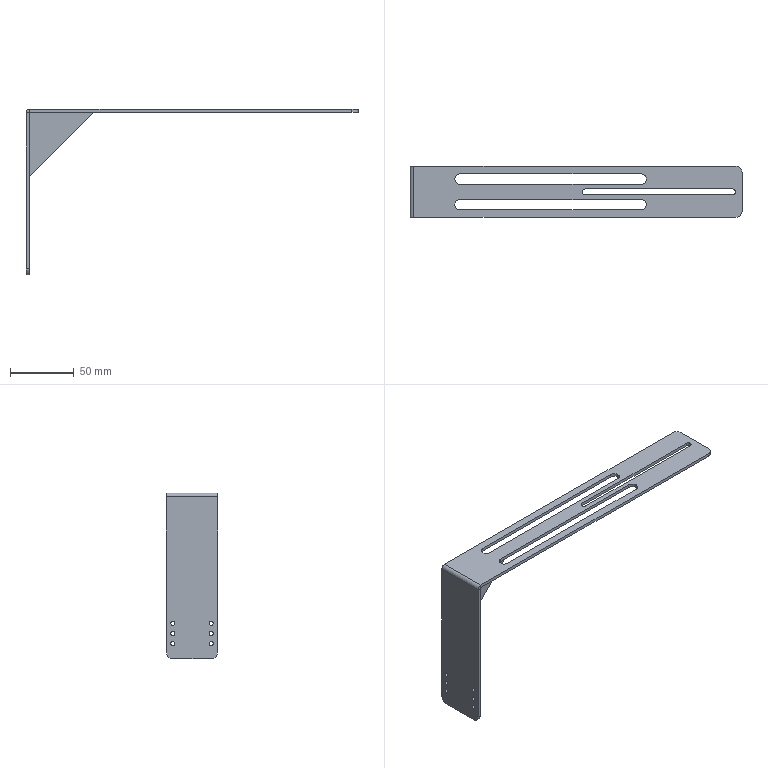Part | SolidWorks | features HoleWzd 3, EdgeFlange 1, Fillet 1, FlatPattern 1, ICE 1, SMBaseFlange 1, SheetMetal 1 | 1 solid | 49 faces | box 260 x 40 x 130 mm | volume 34410 mm3 | cylinder 28 | plane 21 | commonest cylinder face diameters 3.3 x12 8 x6 10 x4 4.5 x3 1 x2 6 x1
STEP:
#1=CARTESIAN_POINT('',(-127.5,-15.,-111.65));
#2=VERTEX_POINT('',#1);
#3=CARTESIAN_POINT('',(-127.5,-15.,-108.35));
#4=VERTEX_POINT('',#3);
#5=CARTESIAN_POINT('',(-127.5,-15.,-110.));
#6=DIRECTION('',(-1.,0.,0.));
#7=DIRECTION('',(0.,0.,1.));
#8=AXIS2_PLACEMENT_3D('',#5,#6,#7);
#9=CIRCLE('',#8,1.65);
#10=EDGE_CURVE('',#2,#4,#9,.T.);
#11=ORIENTED_EDGE('',*,*,#10,.F.);
#12=CARTESIAN_POINT('',(-130.,-15.,-111.65));
#13=VERTEX_POINT('',#12);
#14=CARTESIAN_POINT('',(-130.,-15.,-111.65));
#15=DIRECTION('',(-1.,0.,0.));
#16=VECTOR('',#15,1000.);
#17=LINE('',#14,#16);
#18=EDGE_CURVE('',#2,#13,#17,.T.);
#19=ORIENTED_EDGE('',*,*,#18,.T.);
#20=CARTESIAN_POINT('',(-130.,-15.,-108.35));
#21=VERTEX_POINT('',#20);
#22=CARTESIAN_POINT('',(-130.,-15.,-110.));
#23=DIRECTION('',(-1.,0.,0.));
#24=DIRECTION('',(0.,0.,1.));
#25=AXIS2_PLACEMENT_3D('',#22,#23,#24);
#26=CIRCLE('',#25,1.65);
#27=EDGE_CURVE('',#13,#21,#26,.T.);
#28=ORIENTED_EDGE('',*,*,#27,.T.);
#29=CARTESIAN_POINT('',(-130.,-15.,-108.35));
#30=DIRECTION('',(-1.,0.,0.));
#31=VECTOR('',#30,1000.);
#32=LINE('',#29,#31);
#33=EDGE_CURVE('',#4,#21,#32,.T.);
#34=ORIENTED_EDGE('',*,*,#33,.F.);
#35=EDGE_LOOP('',(#11,#19,#28,#34));
#36=FACE_OUTER_BOUND('',#35,.T.);
#37=CARTESIAN_POINT('',(-130.,-15.,-110.));
#38=DIRECTION('',(-1.,0.,0.));
#39=DIRECTION('',(0.,0.,1.));
#40=AXIS2_PLACEMENT_3D('',#37,#38,#39);
#41=CYLINDRICAL_SURFACE('',#40,1.65);
#42=ADVANCED_FACE('',(#36),#41,.F.);
#43=CARTESIAN_POINT('',(-127.5,15.,-111.65));
#44=VERTEX_POINT('',#43);
#45=CARTESIAN_POINT('',(-127.5,15.,-108.35));
#46=VERTEX_POINT('',#45);
#47=CARTESIAN_POINT('',(-127.5,15.,-110.));
#48=DIRECTION('',(-1.,0.,0.));
#49=DIRECTION('',(0.,0.,1.));
#50=AXIS2_PLACEMENT_3D('',#47,#48,#49);
#51=CIRCLE('',#50,1.65);
#52=EDGE_CURVE('',#44,#46,#51,.T.);
#53=ORIENTED_EDGE('',*,*,#52,.F.);
#54=CARTESIAN_POINT('',(-130.,15.,-111.65));
#55=VERTEX_POINT('',#54);
#56=CARTESIAN_POINT('',(-130.,15.,-111.65));
#57=DIRECTION('',(-1.,0.,0.));
#58=VECTOR('',#57,1000.);
#59=LINE('',#56,#58);
#60=EDGE_CURVE('',#44,#55,#59,.T.);
#61=ORIENTED_EDGE('',*,*,#60,.T.);
#62=CARTESIAN_POINT('',(-130.,15.,-108.35));
#63=VERTEX_POINT('',#62);
#64=CARTESIAN_POINT('',(-130.,15.,-110.));
#65=DIRECTION('',(-1.,0.,0.));
#66=DIRECTION('',(0.,0.,1.));
#67=AXIS2_PLACEMENT_3D('',#64,#65,#66);
#68=CIRCLE('',#67,1.65);
#69=EDGE_CURVE('',#55,#63,#68,.T.);
#70=ORIENTED_EDGE('',*,*,#69,.T.);
#71=CARTESIAN_POINT('',(-130.,15.,-108.35));
#72=DIRECTION('',(-1.,0.,0.));
#73=VECTOR('',#72,1000.);
#74=LINE('',#71,#73);
#75=EDGE_CURVE('',#46,#63,#74,.T.);
#76=ORIENTED_EDGE('',*,*,#75,.F.);
#77=EDGE_LOOP('',(#53,#61,#70,#76));
#78=FACE_OUTER_BOUND('',#77,.T.);
#79=CARTESIAN_POINT('',(-130.,15.,-110.));
#80=DIRECTION('',(-1.,0.,0.));
#81=DIRECTION('',(0.,0.,1.));
#82=AXIS2_PLACEMENT_3D('',#79,#80,#81);
#83=CYLINDRICAL_SURFACE('',#82,1.65);
#84=ADVANCED_FACE('',(#78),#83,.F.);
#85=CARTESIAN_POINT('',(-127.5,-15.,-103.65));
#86=VERTEX_POINT('',#85);
#87=CARTESIAN_POINT('',(-127.5,-15.,-100.35));
#88=VERTEX_POINT('',#87);
#89=CARTESIAN_POINT('',(-127.5,-15.,-102.));
#90=DIRECTION('',(-1.,0.,0.));
#91=DIRECTION('',(0.,0.,1.));
#92=AXIS2_PLACEMENT_3D('',#89,#90,#91);
#93=CIRCLE('',#92,1.65);
#94=EDGE_CURVE('',#86,#88,#93,.T.);
#95=ORIENTED_EDGE('',*,*,#94,.F.);
#96=CARTESIAN_POINT('',(-130.,-15.,-103.65));
#97=VERTEX_POINT('',#96);
#98=CARTESIAN_POINT('',(-130.,-15.,-103.65));
#99=DIRECTION('',(-1.,0.,0.));
#100=VECTOR('',#99,1000.);
#101=LINE('',#98,#100);
#102=EDGE_CURVE('',#86,#97,#101,.T.);
#103=ORIENTED_EDGE('',*,*,#102,.T.);
#104=CARTESIAN_POINT('',(-130.,-15.,-100.35));
#105=VERTEX_POINT('',#104);
#106=CARTESIAN_POINT('',(-130.,-15.,-102.));
#107=DIRECTION('',(-1.,0.,0.));
#108=DIRECTION('',(0.,0.,1.));
#109=AXIS2_PLACEMENT_3D('',#106,#107,#108);
#110=CIRCLE('',#109,1.65);
#111=EDGE_CURVE('',#97,#105,#110,.T.);
#112=ORIENTED_EDGE('',*,*,#111,.T.);
#113=CARTESIAN_POINT('',(-130.,-15.,-100.35));
#114=DIRECTION('',(-1.,0.,0.));
#115=VECTOR('',#114,1000.);
#116=LINE('',#113,#115);
#117=EDGE_CURVE('',#88,#105,#116,.T.);
#118=ORIENTED_EDGE('',*,*,#117,.F.);
#119=EDGE_LOOP('',(#95,#103,#112,#118));
#120=FACE_OUTER_BOUND('',#119,.T.);
#121=CARTESIAN_POINT('',(-130.,-15.,-102.));
#122=DIRECTION('',(-1.,0.,0.));
#123=DIRECTION('',(0.,0.,1.));
#124=AXIS2_PLACEMENT_3D('',#121,#122,#123);
#125=CYLINDRICAL_SURFACE('',#124,1.65);
#126=ADVANCED_FACE('',(#120),#125,.F.);
#127=CARTESIAN_POINT('',(-127.5,15.,-103.65));
#128=VERTEX_POINT('',#127);
#129=CARTESIAN_POINT('',(-127.5,15.,-100.35));
#130=VERTEX_POINT('',#129);
#131=CARTESIAN_POINT('',(-127.5,15.,-102.));
#132=DIRECTION('',(-1.,0.,0.));
#133=DIRECTION('',(0.,0.,1.));
#134=AXIS2_PLACEMENT_3D('',#131,#132,#133);
#135=CIRCLE('',#134,1.65);
#136=EDGE_CURVE('',#128,#130,#135,.T.);
#137=ORIENTED_EDGE('',*,*,#136,.F.);
#138=CARTESIAN_POINT('',(-130.,15.,-103.65));
#139=VERTEX_POINT('',#138);
#140=CARTESIAN_POINT('',(-130.,15.,-103.65));
#141=DIRECTION('',(-1.,0.,0.));
#142=VECTOR('',#141,1000.);
#143=LINE('',#140,#142);
#144=EDGE_CURVE('',#128,#139,#143,.T.);
#145=ORIENTED_EDGE('',*,*,#144,.T.);
#146=CARTESIAN_POINT('',(-130.,15.,-100.35));
#147=VERTEX_POINT('',#146);
#148=CARTESIAN_POINT('',(-130.,15.,-102.));
#149=DIRECTION('',(-1.,0.,0.));
#150=DIRECTION('',(0.,0.,1.));
#151=AXIS2_PLACEMENT_3D('',#148,#149,#150);
#152=CIRCLE('',#151,1.65);
#153=EDGE_CURVE('',#139,#147,#152,.T.);
#154=ORIENTED_EDGE('',*,*,#153,.T.);
#155=CARTESIAN_POINT('',(-130.,15.,-100.35));
#156=DIRECTION('',(-1.,0.,0.));
#157=VECTOR('',#156,1000.);
#158=LINE('',#155,#157);
#159=EDGE_CURVE('',#130,#147,#158,.T.);
#160=ORIENTED_EDGE('',*,*,#159,.F.);
#161=EDGE_LOOP('',(#137,#145,#154,#160));
#162=FACE_OUTER_BOUND('',#161,.T.);
#163=CARTESIAN_POINT('',(-130.,15.,-102.));
#164=DIRECTION('',(-1.,0.,0.));
#165=DIRECTION('',(0.,0.,1.));
#166=AXIS2_PLACEMENT_3D('',#163,#164,#165);
#167=CYLINDRICAL_SURFACE('',#166,1.65);
#168=ADVANCED_FACE('',(#162),#167,.F.);
#169=CARTESIAN_POINT('',(-127.5,-15.,-119.65));
#170=VERTEX_POINT('',#169);
#171=CARTESIAN_POINT('',(-127.5,-15.,-116.35));
#172=VERTEX_POINT('',#171);
#173=CARTESIAN_POINT('',(-127.5,-15.,-118.));
#174=DIRECTION('',(-1.,0.,0.));
#175=DIRECTION('',(0.,0.,1.));
#176=AXIS2_PLACEMENT_3D('',#173,#174,#175);
#177=CIRCLE('',#176,1.65);
#178=EDGE_CURVE('',#170,#172,#177,.T.);
#179=ORIENTED_EDGE('',*,*,#178,.F.);
#180=CARTESIAN_POINT('',(-130.,-15.,-119.65));
#181=VERTEX_POINT('',#180);
#182=CARTESIAN_POINT('',(-130.,-15.,-119.65));
#183=DIRECTION('',(-1.,0.,0.));
#184=VECTOR('',#183,1000.);
#185=LINE('',#182,#184);
#186=EDGE_CURVE('',#170,#181,#185,.T.);
#187=ORIENTED_EDGE('',*,*,#186,.T.);
#188=CARTESIAN_POINT('',(-130.,-15.,-116.35));
#189=VERTEX_POINT('',#188);
#190=CARTESIAN_POINT('',(-130.,-15.,-118.));
#191=DIRECTION('',(-1.,0.,0.));
#192=DIRECTION('',(0.,0.,1.));
#193=AXIS2_PLACEMENT_3D('',#190,#191,#192);
#194=CIRCLE('',#193,1.65);
#195=EDGE_CURVE('',#181,#189,#194,.T.);
#196=ORIENTED_EDGE('',*,*,#195,.T.);
#197=CARTESIAN_POINT('',(-130.,-15.,-116.35));
#198=DIRECTION('',(-1.,0.,0.));
#199=VECTOR('',#198,1000.);
#200=LINE('',#197,#199);
#201=EDGE_CURVE('',#172,#189,#200,.T.);
#202=ORIENTED_EDGE('',*,*,#201,.F.);
#203=EDGE_LOOP('',(#179,#187,#196,#202));
#204=FACE_OUTER_BOUND('',#203,.T.);
#205=CARTESIAN_POINT('',(-130.,-15.,-118.));
#206=DIRECTION('',(-1.,0.,0.));
#207=DIRECTION('',(0.,0.,1.));
#208=AXIS2_PLACEMENT_3D('',#205,#206,#207);
#209=CYLINDRICAL_SURFACE('',#208,1.65);
#210=ADVANCED_FACE('',(#204),#209,.F.);
#211=CARTESIAN_POINT('',(-127.5,15.,-119.65));
#212=VERTEX_POINT('',#211);
#213=CARTESIAN_POINT('',(-127.5,15.,-116.35));
#214=VERTEX_POINT('',#213);
#215=CARTESIAN_POINT('',(-127.5,15.,-118.));
#216=DIRECTION('',(-1.,0.,0.));
#217=DIRECTION('',(0.,0.,1.));
#218=AXIS2_PLACEMENT_3D('',#215,#216,#217);
#219=CIRCLE('',#218,1.65);
#220=EDGE_CURVE('',#212,#214,#219,.T.);
#221=ORIENTED_EDGE('',*,*,#220,.F.);
#222=CARTESIAN_POINT('',(-130.,15.,-119.65));
#223=VERTEX_POINT('',#222);
#224=CARTESIAN_POINT('',(-130.,15.,-119.65));
#225=DIRECTION('',(-1.,0.,0.));
#226=VECTOR('',#225,1000.);
#227=LINE('',#224,#226);
#228=EDGE_CURVE('',#212,#223,#227,.T.);
#229=ORIENTED_EDGE('',*,*,#228,.T.);
#230=CARTESIAN_POINT('',(-130.,15.,-116.35));
#231=VERTEX_POINT('',#230);
#232=CARTESIAN_POINT('',(-130.,15.,-118.));
#233=DIRECTION('',(-1.,0.,0.));
#234=DIRECTION('',(0.,0.,1.));
#235=AXIS2_PLACEMENT_3D('',#232,#233,#234);
#236=CIRCLE('',#235,1.65);
#237=EDGE_CURVE('',#223,#231,#236,.T.);
#238=ORIENTED_EDGE('',*,*,#237,.T.);
#239=CARTESIAN_POINT('',(-130.,15.,-116.35));
#240=DIRECTION('',(-1.,0.,0.));
#241=VECTOR('',#240,1000.);
#242=LINE('',#239,#241);
#243=EDGE_CURVE('',#214,#231,#242,.T.);
#244=ORIENTED_EDGE('',*,*,#243,.F.);
#245=EDGE_LOOP('',(#221,#229,#238,#244));
#246=FACE_OUTER_BOUND('',#245,.T.);
#247=CARTESIAN_POINT('',(-130.,15.,-118.));
#248=DIRECTION('',(-1.,0.,0.));
#249=DIRECTION('',(0.,0.,1.));
#250=AXIS2_PLACEMENT_3D('',#247,#248,#249);
#251=CYLINDRICAL_SURFACE('',#250,1.65);
#252=ADVANCED_FACE('',(#246),#251,.F.);
#253=CARTESIAN_POINT('',(125.,0.,-2.5));
#254=VERTEX_POINT('',#253);
#255=CARTESIAN_POINT('',(122.75,2.25,-2.5));
#256=VERTEX_POINT('',#255);
#257=CARTESIAN_POINT('',(122.75,0.,-2.5));
#258=DIRECTION('',(0.,0.,1.));
#259=DIRECTION('',(1.,0.,0.));
#260=AXIS2_PLACEMENT_3D('',#257,#258,#259);
#261=CIRCLE('',#260,2.25);
#262=EDGE_CURVE('',#254,#256,#261,.T.);
#263=ORIENTED_EDGE('',*,*,#262,.F.);
#264=CARTESIAN_POINT('',(125.,0.,0.));
#265=VERTEX_POINT('',#264);
#266=CARTESIAN_POINT('',(125.,0.,0.));
#267=DIRECTION('',(0.,0.,1.));
#268=VECTOR('',#267,1000.);
#269=LINE('',#266,#268);
#270=EDGE_CURVE('',#254,#265,#269,.T.);
#271=ORIENTED_EDGE('',*,*,#270,.T.);
#272=CARTESIAN_POINT('',(122.75,2.25,0.));
#273=VERTEX_POINT('',#272);
#274=CARTESIAN_POINT('',(122.75,0.,0.));
#275=DIRECTION('',(0.,0.,1.));
#276=DIRECTION('',(1.,0.,0.));
#277=AXIS2_PLACEMENT_3D('',#274,#275,#276);
#278=CIRCLE('',#277,2.25);
#279=EDGE_CURVE('',#265,#273,#278,.T.);
#280=ORIENTED_EDGE('',*,*,#279,.T.);
#281=CARTESIAN_POINT('',(122.75,2.25,0.));
#282=DIRECTION('',(0.,0.,1.));
#283=VECTOR('',#282,1000.);
#284=LINE('',#281,#283);
#285=EDGE_CURVE('',#256,#273,#284,.T.);
#286=ORIENTED_EDGE('',*,*,#285,.F.);
#287=EDGE_LOOP('',(#263,#271,#280,#286));
#288=FACE_OUTER_BOUND('',#287,.T.);
#289=CARTESIAN_POINT('',(122.75,0.,0.));
#290=DIRECTION('',(0.,0.,1.));
#291=DIRECTION('',(1.,0.,0.));
#292=AXIS2_PLACEMENT_3D('',#289,#290,#291);
#293=CYLINDRICAL_SURFACE('',#292,2.25);
#294=ADVANCED_FACE('',(#288),#293,.F.);
#295=CARTESIAN_POINT('',(55.,10.,-2.5));
#296=VERTEX_POINT('',#295);
#297=CARTESIAN_POINT('',(51.,14.,-2.5));
#298=VERTEX_POINT('',#297);
#299=CARTESIAN_POINT('',(51.,10.,-2.5));
#300=DIRECTION('',(0.,0.,1.));
#301=DIRECTION('',(1.,0.,0.));
#302=AXIS2_PLACEMENT_3D('',#299,#300,#301);
#303=CIRCLE('',#302,4.);
#304=EDGE_CURVE('',#296,#298,#303,.T.);
#305=ORIENTED_EDGE('',*,*,#304,.F.);
#306=CARTESIAN_POINT('',(55.,10.,0.));
#307=VERTEX_POINT('',#306);
#308=CARTESIAN_POINT('',(55.,10.,0.));
#309=DIRECTION('',(0.,0.,1.));
#310=VECTOR('',#309,1000.);
#311=LINE('',#308,#310);
#312=EDGE_CURVE('',#296,#307,#311,.T.);
#313=ORIENTED_EDGE('',*,*,#312,.T.);
#314=CARTESIAN_POINT('',(51.,14.,0.));
#315=VERTEX_POINT('',#314);
#316=CARTESIAN_POINT('',(51.,10.,0.));
#317=DIRECTION('',(0.,0.,1.));
#318=DIRECTION('',(1.,0.,0.));
#319=AXIS2_PLACEMENT_3D('',#316,#317,#318);
#320=CIRCLE('',#319,4.);
#321=EDGE_CURVE('',#307,#315,#320,.T.);
#322=ORIENTED_EDGE('',*,*,#321,.T.);
#323=CARTESIAN_POINT('',(51.,14.,0.));
#324=DIRECTION('',(0.,0.,1.));
#325=VECTOR('',#324,1000.);
#326=LINE('',#323,#325);
#327=EDGE_CURVE('',#298,#315,#326,.T.);
#328=ORIENTED_EDGE('',*,*,#327,.F.);
#329=EDGE_LOOP('',(#305,#313,#322,#328));
#330=FACE_OUTER_BOUND('',#329,.T.);
#331=CARTESIAN_POINT('',(51.,10.,0.));
#332=DIRECTION('',(0.,0.,1.));
#333=DIRECTION('',(1.,0.,0.));
#334=AXIS2_PLACEMENT_3D('',#331,#332,#333);
#335=CYLINDRICAL_SURFACE('',#334,4.);
#336=ADVANCED_FACE('',(#330),#335,.F.);
#337=CARTESIAN_POINT('',(55.,-10.,-2.5));
#338=VERTEX_POINT('',#337);
#339=CARTESIAN_POINT('',(51.,-6.,-2.5));
#340=VERTEX_POINT('',#339);
#341=CARTESIAN_POINT('',(51.,-10.,-2.5));
#342=DIRECTION('',(0.,0.,1.));
#343=DIRECTION('',(1.,0.,0.));
#344=AXIS2_PLACEMENT_3D('',#341,#342,#343);
#345=CIRCLE('',#344,4.);
#346=EDGE_CURVE('',#338,#340,#345,.T.);
#347=ORIENTED_EDGE('',*,*,#346,.F.);
#348=CARTESIAN_POINT('',(55.,-10.,0.));
#349=VERTEX_POINT('',#348);
#350=CARTESIAN_POINT('',(55.,-10.,0.));
#351=DIRECTION('',(0.,0.,1.));
#352=VECTOR('',#351,1000.);
#353=LINE('',#350,#352);
#354=EDGE_CURVE('',#338,#349,#353,.T.);
#355=ORIENTED_EDGE('',*,*,#354,.T.);
#356=CARTESIAN_POINT('',(51.,-6.,0.));
#357=VERTEX_POINT('',#356);
#358=CARTESIAN_POINT('',(51.,-10.,0.));
#359=DIRECTION('',(0.,0.,1.));
#360=DIRECTION('',(1.,0.,0.));
#361=AXIS2_PLACEMENT_3D('',#358,#359,#360);
#362=CIRCLE('',#361,4.);
#363=EDGE_CURVE('',#349,#357,#362,.T.);
#364=ORIENTED_EDGE('',*,*,#363,.T.);
#365=CARTESIAN_POINT('',(51.,-6.,0.));
#366=DIRECTION('',(0.,0.,1.));
#367=VECTOR('',#366,1000.);
#368=LINE('',#365,#367);
#369=EDGE_CURVE('',#340,#357,#368,.T.);
#370=ORIENTED_EDGE('',*,*,#369,.F.);
#371=EDGE_LOOP('',(#347,#355,#364,#370));
#372=FACE_OUTER_BOUND('',#371,.T.);
#373=CARTESIAN_POINT('',(51.,-10.,0.));
#374=DIRECTION('',(0.,0.,1.));
#375=DIRECTION('',(1.,0.,0.));
#376=AXIS2_PLACEMENT_3D('',#373,#374,#375);
#377=CYLINDRICAL_SURFACE('',#376,4.);
#378=ADVANCED_FACE('',(#372),#377,.F.);
#379=CARTESIAN_POINT('',(-127.5,-1.25,-3.));
#380=VERTEX_POINT('',#379);
#381=CARTESIAN_POINT('',(-127.,-1.25,-2.5));
#382=VERTEX_POINT('',#381);
#383=CARTESIAN_POINT('',(-127.,-1.25,-3.));
#384=DIRECTION('',(0.,1.,0.));
#385=DIRECTION('',(0.,0.,1.));
#386=AXIS2_PLACEMENT_3D('',#383,#384,#385);
#387=CIRCLE('',#386,0.5);
#388=EDGE_CURVE('',#380,#382,#387,.T.);
#389=ORIENTED_EDGE('',*,*,#388,.T.);
#390=CARTESIAN_POINT('',(-127.,-20.,-2.5));
#391=VERTEX_POINT('',#390);
#392=CARTESIAN_POINT('',(-127.,20.,-2.5));
#393=DIRECTION('',(0.,-1.,0.));
#394=VECTOR('',#393,1000.);
#395=LINE('',#392,#394);
#396=EDGE_CURVE('',#382,#391,#395,.T.);
#397=ORIENTED_EDGE('',*,*,#396,.T.);
#398=CARTESIAN_POINT('',(-127.5,-20.,-3.));
#399=VERTEX_POINT('',#398);
#400=CARTESIAN_POINT('',(-127.,-20.,-3.));
#401=DIRECTION('',(0.,-1.,0.));
#402=DIRECTION('',(0.,0.,1.));
#403=AXIS2_PLACEMENT_3D('',#400,#401,#402);
#404=CIRCLE('',#403,0.5);
#405=EDGE_CURVE('',#391,#399,#404,.T.);
#406=ORIENTED_EDGE('',*,*,#405,.T.);
#407=CARTESIAN_POINT('',(-127.5,-20.,-3.));
#408=DIRECTION('',(0.,1.,0.));
#409=VECTOR('',#408,1000.);
#410=LINE('',#407,#409);
#411=EDGE_CURVE('',#399,#380,#410,.T.);
#412=ORIENTED_EDGE('',*,*,#411,.T.);
#413=EDGE_LOOP('',(#389,#397,#406,#412));
#414=FACE_OUTER_BOUND('',#413,.T.);
#415=CARTESIAN_POINT('',(-127.,20.,-3.));
#416=DIRECTION('',(0.,1.,0.));
#417=DIRECTION('',(-1.,0.,0.));
#418=AXIS2_PLACEMENT_3D('',#415,#416,#417);
#419=CYLINDRICAL_SURFACE('',#418,0.5);
#420=ADVANCED_FACE('',(#414),#419,.F.);
#421=CARTESIAN_POINT('',(-91.,6.,0.));
#422=VERTEX_POINT('',#421);
#423=CARTESIAN_POINT('',(51.,6.,0.));
#424=VERTEX_POINT('',#423);
#425=CARTESIAN_POINT('',(-91.,6.,0.));
#426=DIRECTION('',(1.,0.,0.));
#427=VECTOR('',#426,1000.);
#428=LINE('',#425,#427);
#429=EDGE_CURVE('',#422,#424,#428,.T.);
#430=ORIENTED_EDGE('',*,*,#429,.F.);
#431=CARTESIAN_POINT('',(-91.,14.,0.));
#432=VERTEX_POINT('',#431);
#433=CARTESIAN_POINT('',(-91.,10.,0.));
#434=DIRECTION('',(0.,0.,1.));
#435=DIRECTION('',(1.,0.,0.));
#436=AXIS2_PLACEMENT_3D('',#433,#434,#435);
#437=CIRCLE('',#436,4.);
#438=EDGE_CURVE('',#432,#422,#437,.T.);
#439=ORIENTED_EDGE('',*,*,#438,.F.);
#440=CARTESIAN_POINT('',(-91.,14.,0.));
#441=DIRECTION('',(1.,0.,0.));
#442=VECTOR('',#441,1000.);
#443=LINE('',#440,#442);
#444=EDGE_CURVE('',#432,#315,#443,.T.);
#445=ORIENTED_EDGE('',*,*,#444,.T.);
#446=ORIENTED_EDGE('',*,*,#321,.F.);
#447=CARTESIAN_POINT('',(51.,10.,0.));
#448=DIRECTION('',(0.,0.,1.));
#449=DIRECTION('',(1.,0.,0.));
#450=AXIS2_PLACEMENT_3D('',#447,#448,#449);
#451=CIRCLE('',#450,4.);
#452=EDGE_CURVE('',#424,#307,#451,.T.);
#453=ORIENTED_EDGE('',*,*,#452,.F.);
#454=EDGE_LOOP('',(#430,#439,#445,#446,#453));
#455=FACE_BOUND('',#454,.T.);
#456=CARTESIAN_POINT('',(51.,-14.,0.));
#457=VERTEX_POINT('',#456);
#458=CARTESIAN_POINT('',(51.,-10.,0.));
#459=DIRECTION('',(0.,0.,1.));
#460=DIRECTION('',(1.,0.,0.));
#461=AXIS2_PLACEMENT_3D('',#458,#459,#460);
#462=CIRCLE('',#461,4.);
#463=EDGE_CURVE('',#457,#349,#462,.T.);
#464=ORIENTED_EDGE('',*,*,#463,.F.);
#465=CARTESIAN_POINT('',(-91.,-14.,0.));
#466=VERTEX_POINT('',#465);
#467=CARTESIAN_POINT('',(-91.,-14.,0.));
#468=DIRECTION('',(1.,0.,0.));
#469=VECTOR('',#468,1000.);
#470=LINE('',#467,#469);
#471=EDGE_CURVE('',#466,#457,#470,.T.);
#472=ORIENTED_EDGE('',*,*,#471,.F.);
#473=CARTESIAN_POINT('',(-91.,-6.,0.));
#474=VERTEX_POINT('',#473);
#475=CARTESIAN_POINT('',(-91.,-10.,0.));
#476=DIRECTION('',(0.,0.,1.));
#477=DIRECTION('',(1.,0.,0.));
#478=AXIS2_PLACEMENT_3D('',#475,#476,#477);
#479=CIRCLE('',#478,4.);
#480=EDGE_CURVE('',#474,#466,#479,.T.);
#481=ORIENTED_EDGE('',*,*,#480,.F.);
#482=CARTESIAN_POINT('',(-91.,-6.,0.));
#483=DIRECTION('',(1.,0.,0.));
#484=VECTOR('',#483,1000.);
#485=LINE('',#482,#484);
#486=EDGE_CURVE('',#474,#357,#485,.T.);
#487=ORIENTED_EDGE('',*,*,#486,.T.);
#488=ORIENTED_EDGE('',*,*,#363,.F.);
#489=EDGE_LOOP('',(#464,#472,#481,#487,#488));
#490=FACE_BOUND('',#489,.T.);
#491=CARTESIAN_POINT('',(130.,-15.,0.));
#492=VERTEX_POINT('',#491);
#493=CARTESIAN_POINT('',(130.,15.,0.));
#494=VERTEX_POINT('',#493);
#495=CARTESIAN_POINT('',(130.,20.,0.));
#496=DIRECTION('',(0.,1.,0.));
#497=VECTOR('',#496,1000.);
#498=LINE('',#495,#497);
#499=EDGE_CURVE('',#492,#494,#498,.T.);
#500=ORIENTED_EDGE('',*,*,#499,.T.);
#501=CARTESIAN_POINT('',(125.,20.,0.));
#502=VERTEX_POINT('',#501);
#503=CARTESIAN_POINT('',(125.,15.,0.));
#504=DIRECTION('',(0.,0.,1.));
#505=DIRECTION('',(1.,0.,0.));
#506=AXIS2_PLACEMENT_3D('',#503,#504,#505);
#507=CIRCLE('',#506,5.);
#508=EDGE_CURVE('',#494,#502,#507,.T.);
#509=ORIENTED_EDGE('',*,*,#508,.T.);
#510=CARTESIAN_POINT('',(-127.,20.,0.));
#511=VERTEX_POINT('',#510);
#512=CARTESIAN_POINT('',(-130.,20.,0.));
#513=DIRECTION('',(-1.,0.,0.));
#514=VECTOR('',#513,1000.);
#515=LINE('',#512,#514);
#516=EDGE_CURVE('',#502,#511,#515,.T.);
#517=ORIENTED_EDGE('',*,*,#516,.T.);
#518=CARTESIAN_POINT('',(-127.,-20.,0.));
#519=VERTEX_POINT('',#518);
#520=CARTESIAN_POINT('',(-127.,20.,0.));
#521=DIRECTION('',(0.,-1.,0.));
#522=VECTOR('',#521,1000.);
#523=LINE('',#520,#522);
#524=EDGE_CURVE('',#511,#519,#523,.T.);
#525=ORIENTED_EDGE('',*,*,#524,.T.);
#526=CARTESIAN_POINT('',(125.,-20.,0.));
#527=VERTEX_POINT('',#526);
#528=CARTESIAN_POINT('',(-130.,-20.,0.));
#529=DIRECTION('',(1.,0.,0.));
#530=VECTOR('',#529,1000.);
#531=LINE('',#528,#530);
#532=EDGE_CURVE('',#519,#527,#531,.T.);
#533=ORIENTED_EDGE('',*,*,#532,.T.);
#534=CARTESIAN_POINT('',(125.,-15.,0.));
#535=DIRECTION('',(0.,0.,1.));
#536=DIRECTION('',(1.,0.,0.));
#537=AXIS2_PLACEMENT_3D('',#534,#535,#536);
#538=CIRCLE('',#537,5.);
#539=EDGE_CURVE('',#527,#492,#538,.T.);
#540=ORIENTED_EDGE('',*,*,#539,.T.);
#541=EDGE_LOOP('',(#500,#509,#517,#525,#533,#540));
#542=FACE_OUTER_BOUND('',#541,.T.);
#543=CARTESIAN_POINT('',(7.25,2.25,0.));
#544=VERTEX_POINT('',#543);
#545=CARTESIAN_POINT('',(7.25,-2.25,0.));
#546=VERTEX_POINT('',#545);
#547=CARTESIAN_POINT('',(7.25,0.,0.));
#548=DIRECTION('',(0.,0.,1.));
#549=DIRECTION('',(1.,0.,0.));
#550=AXIS2_PLACEMENT_3D('',#547,#548,#549);
#551=CIRCLE('',#550,2.25);
#552=EDGE_CURVE('',#544,#546,#551,.T.);
#553=ORIENTED_EDGE('',*,*,#552,.F.);
#554=CARTESIAN_POINT('',(7.25,2.25,0.));
#555=DIRECTION('',(1.,0.,0.));
#556=VECTOR('',#555,1000.);
#557=LINE('',#554,#556);
#558=EDGE_CURVE('',#544,#273,#557,.T.);
#559=ORIENTED_EDGE('',*,*,#558,.T.);
#560=ORIENTED_EDGE('',*,*,#279,.F.);
#561=CARTESIAN_POINT('',(122.75,-2.25,0.));
#562=VERTEX_POINT('',#561);
#563=CARTESIAN_POINT('',(122.75,0.,0.));
#564=DIRECTION('',(0.,0.,1.));
#565=DIRECTION('',(1.,0.,0.));
#566=AXIS2_PLACEMENT_3D('',#563,#564,#565);
#567=CIRCLE('',#566,2.25);
#568=EDGE_CURVE('',#562,#265,#567,.T.);
#569=ORIENTED_EDGE('',*,*,#568,.F.);
#570=CARTESIAN_POINT('',(7.25,-2.25,0.));
#571=DIRECTION('',(1.,0.,0.));
#572=VECTOR('',#571,1000.);
#573=LINE('',#570,#572);
#574=EDGE_CURVE('',#546,#562,#573,.T.);
#575=ORIENTED_EDGE('',*,*,#574,.F.);
#576=EDGE_LOOP('',(#553,#559,#560,#569,#575));
#577=FACE_BOUND('',#576,.T.);
#578=CARTESIAN_POINT('',(0.,0.,0.));
#579=DIRECTION('',(0.,0.,1.));
#580=DIRECTION('',(1.,0.,0.));
#581=AXIS2_PLACEMENT_3D('',#578,#579,#580);
#582=PLANE('',#581);
#583=ADVANCED_FACE('',(#455,#490,#542,#577),#582,.T.);
#584=ORIENTED_EDGE('',*,*,#516,.F.);
#585=CARTESIAN_POINT('',(125.,20.,-2.5));
#586=VERTEX_POINT('',#585);
#587=CARTESIAN_POINT('',(125.,20.,-2.5));
#588=DIRECTION('',(0.,0.,-1.));
#589=VECTOR('',#588,1000.);
#590=LINE('',#587,#589);
#591=EDGE_CURVE('',#502,#586,#590,.T.);
#592=ORIENTED_EDGE('',*,*,#591,.T.);
#593=CARTESIAN_POINT('',(-127.,20.,-2.5));
#594=VERTEX_POINT('',#593);
#595=CARTESIAN_POINT('',(-130.,20.,-2.5));
#596=DIRECTION('',(-1.,0.,0.));
#597=VECTOR('',#596,1000.);
#598=LINE('',#595,#597);
#599=EDGE_CURVE('',#586,#594,#598,.T.);
#600=ORIENTED_EDGE('',*,*,#599,.T.);
#601=CARTESIAN_POINT('',(-127.,20.,-2.5));
#602=DIRECTION('',(0.,0.,1.));
#603=VECTOR('',#602,1000.);
#604=LINE('',#601,#603);
#605=EDGE_CURVE('',#594,#511,#604,.T.);
#606=ORIENTED_EDGE('',*,*,#605,.T.);
#607=EDGE_LOOP('',(#584,#592,#600,#606));
#608=FACE_OUTER_BOUND('',#607,.T.);
#609=CARTESIAN_POINT('',(-130.,20.,-2.5));
#610=DIRECTION('',(0.,1.,0.));
#611=DIRECTION('',(0.,0.,1.));
#612=AXIS2_PLACEMENT_3D('',#609,#610,#611);
#613=PLANE('',#612);
#614=ADVANCED_FACE('',(#608),#613,.T.);
#615=CARTESIAN_POINT('',(122.75,-2.25,-2.5));
#616=VERTEX_POINT('',#615);
#617=CARTESIAN_POINT('',(122.75,0.,-2.5));
#618=DIRECTION('',(0.,0.,1.));
#619=DIRECTION('',(1.,0.,0.));
#620=AXIS2_PLACEMENT_3D('',#617,#618,#619);
#621=CIRCLE('',#620,2.25);
#622=EDGE_CURVE('',#616,#254,#621,.T.);
#623=ORIENTED_EDGE('',*,*,#622,.T.);
#624=ORIENTED_EDGE('',*,*,#262,.T.);
#625=CARTESIAN_POINT('',(7.25,2.25,-2.5));
#626=VERTEX_POINT('',#625);
#627=CARTESIAN_POINT('',(0.,2.25,-2.5));
#628=DIRECTION('',(-1.,0.,0.));
#629=VECTOR('',#628,1000.);
#630=LINE('',#627,#629);
#631=EDGE_CURVE('',#256,#626,#630,.T.);
#632=ORIENTED_EDGE('',*,*,#631,.T.);
#633=CARTESIAN_POINT('',(7.25,-2.25,-2.5));
#634=VERTEX_POINT('',#633);
#635=CARTESIAN_POINT('',(7.25,0.,-2.5));
#636=DIRECTION('',(0.,0.,1.));
#637=DIRECTION('',(1.,0.,0.));
#638=AXIS2_PLACEMENT_3D('',#635,#636,#637);
#639=CIRCLE('',#638,2.25);
#640=EDGE_CURVE('',#626,#634,#639,.T.);
#641=ORIENTED_EDGE('',*,*,#640,.T.);
#642=CARTESIAN_POINT('',(0.,-2.25,-2.5));
#643=DIRECTION('',(1.,0.,0.));
#644=VECTOR('',#643,1000.);
#645=LINE('',#642,#644);
#646=EDGE_CURVE('',#634,#616,#645,.T.);
#647=ORIENTED_EDGE('',*,*,#646,.T.);
#648=EDGE_LOOP('',(#623,#624,#632,#641,#647));
#649=FACE_BOUND('',#648,.T.);
#650=CARTESIAN_POINT('',(-91.,14.,-2.5));
#651=VERTEX_POINT('',#650);
#652=CARTESIAN_POINT('',(0.,14.,-2.5));
#653=DIRECTION('',(-1.,0.,0.));
#654=VECTOR('',#653,1000.);
#655=LINE('',#652,#654);
#656=EDGE_CURVE('',#298,#651,#655,.T.);
#657=ORIENTED_EDGE('',*,*,#656,.T.);
#658=CARTESIAN_POINT('',(-91.,6.,-2.5));
#659=VERTEX_POINT('',#658);
#660=CARTESIAN_POINT('',(-91.,10.,-2.5));
#661=DIRECTION('',(0.,0.,1.));
#662=DIRECTION('',(1.,0.,0.));
#663=AXIS2_PLACEMENT_3D('',#660,#661,#662);
#664=CIRCLE('',#663,4.);
#665=EDGE_CURVE('',#651,#659,#664,.T.);
#666=ORIENTED_EDGE('',*,*,#665,.T.);
#667=CARTESIAN_POINT('',(51.,6.,-2.5));
#668=VERTEX_POINT('',#667);
#669=CARTESIAN_POINT('',(0.,6.,-2.5));
#670=DIRECTION('',(1.,0.,0.));
#671=VECTOR('',#670,1000.);
#672=LINE('',#669,#671);
#673=EDGE_CURVE('',#659,#668,#672,.T.);
#674=ORIENTED_EDGE('',*,*,#673,.T.);
#675=CARTESIAN_POINT('',(51.,10.,-2.5));
#676=DIRECTION('',(0.,0.,1.));
#677=DIRECTION('',(1.,0.,0.));
#678=AXIS2_PLACEMENT_3D('',#675,#676,#677);
#679=CIRCLE('',#678,4.);
#680=EDGE_CURVE('',#668,#296,#679,.T.);
#681=ORIENTED_EDGE('',*,*,#680,.T.);
#682=ORIENTED_EDGE('',*,*,#304,.T.);
#683=EDGE_LOOP('',(#657,#666,#674,#681,#682));
#684=FACE_BOUND('',#683,.T.);
#685=CARTESIAN_POINT('',(-91.,-6.,-2.5));
#686=VERTEX_POINT('',#685);
#687=CARTESIAN_POINT('',(0.,-6.,-2.5));
#688=DIRECTION('',(-1.,0.,0.));
#689=VECTOR('',#688,1000.);
#690=LINE('',#687,#689);
#691=EDGE_CURVE('',#340,#686,#690,.T.);
#692=ORIENTED_EDGE('',*,*,#691,.T.);
#693=CARTESIAN_POINT('',(-91.,-14.,-2.5));
#694=VERTEX_POINT('',#693);
#695=CARTESIAN_POINT('',(-91.,-10.,-2.5));
#696=DIRECTION('',(0.,0.,1.));
#697=DIRECTION('',(1.,0.,0.));
#698=AXIS2_PLACEMENT_3D('',#695,#696,#697);
#699=CIRCLE('',#698,4.);
#700=EDGE_CURVE('',#686,#694,#699,.T.);
#701=ORIENTED_EDGE('',*,*,#700,.T.);
#702=CARTESIAN_POINT('',(51.,-14.,-2.5));
#703=VERTEX_POINT('',#702);
#704=CARTESIAN_POINT('',(0.,-14.,-2.5));
#705=DIRECTION('',(1.,0.,0.));
#706=VECTOR('',#705,1000.);
#707=LINE('',#704,#706);
#708=EDGE_CURVE('',#694,#703,#707,.T.);
#709=ORIENTED_EDGE('',*,*,#708,.T.);
#710=CARTESIAN_POINT('',(51.,-10.,-2.5));
#711=DIRECTION('',(0.,0.,1.));
#712=DIRECTION('',(1.,0.,0.));
#713=AXIS2_PLACEMENT_3D('',#710,#711,#712);
#714=CIRCLE('',#713,4.);
#715=EDGE_CURVE('',#703,#338,#714,.T.);
#716=ORIENTED_EDGE('',*,*,#715,.T.);
#717=ORIENTED_EDGE('',*,*,#346,.T.);
#718=EDGE_LOOP('',(#692,#701,#709,#716,#717));
#719=FACE_BOUND('',#718,.T.);
#720=CARTESIAN_POINT('',(-77.,1.25,-2.5));
#721=VERTEX_POINT('',#720);
#722=CARTESIAN_POINT('',(-77.,-1.25,-2.5));
#723=VERTEX_POINT('',#722);
#724=CARTESIAN_POINT('',(-77.,1.25,-2.5));
#725=DIRECTION('',(0.,-1.,0.));
#726=VECTOR('',#725,1000.);
#727=LINE('',#724,#726);
#728=EDGE_CURVE('',#721,#723,#727,.T.);
#729=ORIENTED_EDGE('',*,*,#728,.F.);
#730=CARTESIAN_POINT('',(-127.,1.25,-2.5));
#731=VERTEX_POINT('',#730);
#732=CARTESIAN_POINT('',(-77.,1.25,-2.5));
#733=DIRECTION('',(1.,0.,0.));
#734=VECTOR('',#733,1000.);
#735=LINE('',#732,#734);
#736=EDGE_CURVE('',#731,#721,#735,.T.);
#737=ORIENTED_EDGE('',*,*,#736,.F.);
#738=CARTESIAN_POINT('',(-127.,20.,-2.5));
#739=DIRECTION('',(0.,-1.,0.));
#740=VECTOR('',#739,1000.);
#741=LINE('',#738,#740);
#742=EDGE_CURVE('',#594,#731,#741,.T.);
#743=ORIENTED_EDGE('',*,*,#742,.F.);
#744=ORIENTED_EDGE('',*,*,#599,.F.);
#745=CARTESIAN_POINT('',(130.,15.,-2.5));
#746=VERTEX_POINT('',#745);
#747=CARTESIAN_POINT('',(125.,15.,-2.5));
#748=DIRECTION('',(0.,0.,-1.));
#749=DIRECTION('',(1.,0.,0.));
#750=AXIS2_PLACEMENT_3D('',#747,#748,#749);
#751=CIRCLE('',#750,5.);
#752=EDGE_CURVE('',#586,#746,#751,.T.);
#753=ORIENTED_EDGE('',*,*,#752,.T.);
#754=CARTESIAN_POINT('',(130.,-15.,-2.5));
#755=VERTEX_POINT('',#754);
#756=CARTESIAN_POINT('',(130.,20.,-2.5));
#757=DIRECTION('',(0.,1.,0.));
#758=VECTOR('',#757,1000.);
#759=LINE('',#756,#758);
#760=EDGE_CURVE('',#755,#746,#759,.T.);
#761=ORIENTED_EDGE('',*,*,#760,.F.);
#762=CARTESIAN_POINT('',(125.,-20.,-2.5));
#763=VERTEX_POINT('',#762);
#764=CARTESIAN_POINT('',(125.,-15.,-2.5));
#765=DIRECTION('',(0.,0.,-1.));
#766=DIRECTION('',(1.,0.,0.));
#767=AXIS2_PLACEMENT_3D('',#764,#765,#766);
#768=CIRCLE('',#767,5.);
#769=EDGE_CURVE('',#755,#763,#768,.T.);
#770=ORIENTED_EDGE('',*,*,#769,.T.);
#771=CARTESIAN_POINT('',(-130.,-20.,-2.5));
#772=DIRECTION('',(1.,0.,0.));
#773=VECTOR('',#772,1000.);
#774=LINE('',#771,#773);
#775=EDGE_CURVE('',#391,#763,#774,.T.);
#776=ORIENTED_EDGE('',*,*,#775,.F.);
#777=ORIENTED_EDGE('',*,*,#396,.F.);
#778=CARTESIAN_POINT('',(-77.,-1.25,-2.5));
#779=DIRECTION('',(1.,0.,0.));
#780=VECTOR('',#779,1000.);
#781=LINE('',#778,#780);
#782=EDGE_CURVE('',#382,#723,#781,.T.);
#783=ORIENTED_EDGE('',*,*,#782,.T.);
#784=EDGE_LOOP('',(#729,#737,#743,#744,#753,#761,#770,#776,#777,#783));
#785=FACE_OUTER_BOUND('',#784,.T.);
#786=CARTESIAN_POINT('',(0.,0.,-2.5));
#787=DIRECTION('',(0.,0.,1.));
#788=DIRECTION('',(1.,0.,0.));
#789=AXIS2_PLACEMENT_3D('',#786,#787,#788);
#790=PLANE('',#789);
#791=ADVANCED_FACE('',(#649,#684,#719,#785),#790,.F.);
#792=ORIENTED_EDGE('',*,*,#760,.T.);
#793=CARTESIAN_POINT('',(130.,15.,-2.5));
#794=DIRECTION('',(0.,0.,1.));
#795=VECTOR('',#794,1000.);
#796=LINE('',#793,#795);
#797=EDGE_CURVE('',#746,#494,#796,.T.);
#798=ORIENTED_EDGE('',*,*,#797,.T.);
#799=ORIENTED_EDGE('',*,*,#499,.F.);
#800=CARTESIAN_POINT('',(130.,-15.,-2.5));
#801=DIRECTION('',(0.,0.,-1.));
#802=VECTOR('',#801,1000.);
#803=LINE('',#800,#802);
#804=EDGE_CURVE('',#492,#755,#803,.T.);
#805=ORIENTED_EDGE('',*,*,#804,.T.);
#806=EDGE_LOOP('',(#792,#798,#799,#805));
#807=FACE_OUTER_BOUND('',#806,.T.);
#808=CARTESIAN_POINT('',(130.,20.,-2.5));
#809=DIRECTION('',(1.,0.,0.));
#810=DIRECTION('',(0.,1.,0.));
#811=AXIS2_PLACEMENT_3D('',#808,#809,#810);
#812=PLANE('',#811);
#813=ADVANCED_FACE('',(#807),#812,.T.);
#814=ORIENTED_EDGE('',*,*,#775,.T.);
#815=CARTESIAN_POINT('',(125.,-20.,-2.5));
#816=DIRECTION('',(0.,0.,1.));
#817=VECTOR('',#816,1000.);
#818=LINE('',#815,#817);
#819=EDGE_CURVE('',#763,#527,#818,.T.);
#820=ORIENTED_EDGE('',*,*,#819,.T.);
#821=ORIENTED_EDGE('',*,*,#532,.F.);
#822=CARTESIAN_POINT('',(-127.,-20.,-2.5));
#823=DIRECTION('',(0.,0.,1.));
#824=VECTOR('',#823,1000.);
#825=LINE('',#822,#824);
#826=EDGE_CURVE('',#391,#519,#825,.T.);
#827=ORIENTED_EDGE('',*,*,#826,.F.);
#828=EDGE_LOOP('',(#814,#820,#821,#827));
#829=FACE_OUTER_BOUND('',#828,.T.);
#830=CARTESIAN_POINT('',(-130.,-20.,-2.5));
#831=DIRECTION('',(0.,-1.,0.));
#832=DIRECTION('',(0.,0.,-1.));
#833=AXIS2_PLACEMENT_3D('',#830,#831,#832);
#834=PLANE('',#833);
#835=ADVANCED_FACE('',(#829),#834,.T.);
#836=CARTESIAN_POINT('',(-130.,-20.,-3.));
#837=VERTEX_POINT('',#836);
#838=CARTESIAN_POINT('',(-130.,-20.,-3.));
#839=DIRECTION('',(-1.,0.,0.));
#840=VECTOR('',#839,1000.);
#841=LINE('',#838,#840);
#842=EDGE_CURVE('',#399,#837,#841,.T.);
#843=ORIENTED_EDGE('',*,*,#842,.F.);
#844=ORIENTED_EDGE('',*,*,#405,.F.);
#845=ORIENTED_EDGE('',*,*,#826,.T.);
#846=CARTESIAN_POINT('',(-127.,-20.,-3.));
#847=DIRECTION('',(0.,-1.,0.));
#848=DIRECTION('',(0.,0.,1.));
#849=AXIS2_PLACEMENT_3D('',#846,#847,#848);
#850=CIRCLE('',#849,3.);
#851=EDGE_CURVE('',#519,#837,#850,.T.);
#852=ORIENTED_EDGE('',*,*,#851,.T.);
#853=EDGE_LOOP('',(#843,#844,#845,#852));
#854=FACE_OUTER_BOUND('',#853,.T.);
#855=CARTESIAN_POINT('',(-127.,-20.,-3.));
#856=DIRECTION('',(0.,-1.,0.));
#857=DIRECTION('',(0.,0.,-1.));
#858=AXIS2_PLACEMENT_3D('',#855,#856,#857);
#859=PLANE('',#858);
#860=ADVANCED_FACE('',(#854),#859,.T.);
#861=CARTESIAN_POINT('',(-127.5,20.,-3.));
#862=VERTEX_POINT('',#861);
#863=CARTESIAN_POINT('',(-127.,20.,-3.));
#864=DIRECTION('',(0.,1.,0.));
#865=DIRECTION('',(0.,0.,1.));
#866=AXIS2_PLACEMENT_3D('',#863,#864,#865);
#867=CIRCLE('',#866,0.5);
#868=EDGE_CURVE('',#862,#594,#867,.T.);
#869=ORIENTED_EDGE('',*,*,#868,.F.);
#870=CARTESIAN_POINT('',(-130.,20.,-3.));
#871=VERTEX_POINT('',#870);
#872=CARTESIAN_POINT('',(-127.5,20.,-3.));
#873=DIRECTION('',(-1.,0.,0.));
#874=VECTOR('',#873,1000.);
#875=LINE('',#872,#874);
#876=EDGE_CURVE('',#862,#871,#875,.T.);
#877=ORIENTED_EDGE('',*,*,#876,.T.);
#878=CARTESIAN_POINT('',(-127.,20.,-3.));
#879=DIRECTION('',(0.,1.,0.));
#880=DIRECTION('',(0.,0.,1.));
#881=AXIS2_PLACEMENT_3D('',#878,#879,#880);
#882=CIRCLE('',#881,3.);
#883=EDGE_CURVE('',#871,#511,#882,.T.);
#884=ORIENTED_EDGE('',*,*,#883,.T.);
#885=ORIENTED_EDGE('',*,*,#605,.F.);
#886=EDGE_LOOP('',(#869,#877,#884,#885));
#887=FACE_OUTER_BOUND('',#886,.T.);
#888=CARTESIAN_POINT('',(-127.,20.,-3.));
#889=DIRECTION('',(0.,-1.,0.));
#890=DIRECTION('',(0.,0.,-1.));
#891=AXIS2_PLACEMENT_3D('',#888,#889,#890);
#892=PLANE('',#891);
#893=ADVANCED_FACE('',(#887),#892,.F.);
#894=ORIENTED_EDGE('',*,*,#524,.F.);
#895=ORIENTED_EDGE('',*,*,#883,.F.);
#896=CARTESIAN_POINT('',(-130.,0.,-3.));
#897=DIRECTION('',(0.,1.,0.));
#898=VECTOR('',#897,1000.);
#899=LINE('',#896,#898);
#900=EDGE_CURVE('',#837,#871,#899,.T.);
#901=ORIENTED_EDGE('',*,*,#900,.F.);
#902=ORIENTED_EDGE('',*,*,#851,.F.);
#903=EDGE_LOOP('',(#894,#895,#901,#902));
#904=FACE_OUTER_BOUND('',#903,.T.);
#905=CARTESIAN_POINT('',(-127.,20.,-3.));
#906=DIRECTION('',(0.,1.,0.));
#907=DIRECTION('',(-1.,0.,0.));
#908=AXIS2_PLACEMENT_3D('',#905,#906,#907);
#909=CYLINDRICAL_SURFACE('',#908,3.);
#910=ADVANCED_FACE('',(#904),#909,.T.);
#911=ORIENTED_EDGE('',*,*,#742,.T.);
#912=CARTESIAN_POINT('',(-127.5,1.25,-3.));
#913=VERTEX_POINT('',#912);
#914=CARTESIAN_POINT('',(-127.,1.25,-3.));
#915=DIRECTION('',(0.,1.,0.));
#916=DIRECTION('',(0.,0.,1.));
#917=AXIS2_PLACEMENT_3D('',#914,#915,#916);
#918=CIRCLE('',#917,0.5);
#919=EDGE_CURVE('',#913,#731,#918,.T.);
#920=ORIENTED_EDGE('',*,*,#919,.F.);
#921=CARTESIAN_POINT('',(-127.5,-20.,-3.));
#922=DIRECTION('',(0.,1.,0.));
#923=VECTOR('',#922,1000.);
#924=LINE('',#921,#923);
#925=EDGE_CURVE('',#913,#862,#924,.T.);
#926=ORIENTED_EDGE('',*,*,#925,.T.);
#927=ORIENTED_EDGE('',*,*,#868,.T.);
#928=EDGE_LOOP('',(#911,#920,#926,#927));
#929=FACE_OUTER_BOUND('',#928,.T.);
#930=CARTESIAN_POINT('',(-127.,20.,-3.));
#931=DIRECTION('',(0.,1.,0.));
#932=DIRECTION('',(-1.,0.,0.));
#933=AXIS2_PLACEMENT_3D('',#930,#931,#932);
#934=CYLINDRICAL_SURFACE('',#933,0.5);
#935=ADVANCED_FACE('',(#929),#934,.F.);
#936=CARTESIAN_POINT('',(-127.5,20.,-125.));
#937=VERTEX_POINT('',#936);
#938=CARTESIAN_POINT('',(-127.5,20.,0.));
#939=DIRECTION('',(0.,0.,1.));
#940=VECTOR('',#939,1000.);
#941=LINE('',#938,#940);
#942=EDGE_CURVE('',#937,#862,#941,.T.);
#943=ORIENTED_EDGE('',*,*,#942,.F.);
#944=CARTESIAN_POINT('',(-130.,20.,-125.));
#945=VERTEX_POINT('',#944);
#946=CARTESIAN_POINT('',(-130.,20.,-125.));
#947=DIRECTION('',(-1.,0.,0.));
#948=VECTOR('',#947,1000.);
#949=LINE('',#946,#948);
#950=EDGE_CURVE('',#937,#945,#949,.T.);
#951=ORIENTED_EDGE('',*,*,#950,.T.);
#952=CARTESIAN_POINT('',(-130.,20.,-2.5));
#953=DIRECTION('',(0.,0.,1.));
#954=VECTOR('',#953,1000.);
#955=LINE('',#952,#954);
#956=EDGE_CURVE('',#945,#871,#955,.T.);
#957=ORIENTED_EDGE('',*,*,#956,.T.);
#958=ORIENTED_EDGE('',*,*,#876,.F.);
#959=EDGE_LOOP('',(#943,#951,#957,#958));
#960=FACE_OUTER_BOUND('',#959,.T.);
#961=CARTESIAN_POINT('',(-130.,20.,-2.5));
#962=DIRECTION('',(0.,1.,0.));
#963=DIRECTION('',(0.,0.,1.));
#964=AXIS2_PLACEMENT_3D('',#961,#962,#963);
#965=PLANE('',#964);
#966=ADVANCED_FACE('',(#960),#965,.T.);
#967=CARTESIAN_POINT('',(-130.,-20.,-125.));
#968=VERTEX_POINT('',#967);
#969=CARTESIAN_POINT('',(-130.,-20.,-130.));
#970=DIRECTION('',(0.,0.,-1.));
#971=VECTOR('',#970,1000.);
#972=LINE('',#969,#971);
#973=EDGE_CURVE('',#837,#968,#972,.T.);
#974=ORIENTED_EDGE('',*,*,#973,.T.);
#975=CARTESIAN_POINT('',(-127.5,-20.,-125.));
#976=VERTEX_POINT('',#975);
#977=CARTESIAN_POINT('',(-130.,-20.,-125.));
#978=DIRECTION('',(1.,0.,0.));
#979=VECTOR('',#978,1000.);
#980=LINE('',#977,#979);
#981=EDGE_CURVE('',#968,#976,#980,.T.);
#982=ORIENTED_EDGE('',*,*,#981,.T.);
#983=CARTESIAN_POINT('',(-127.5,-20.,0.));
#984=DIRECTION('',(0.,0.,-1.));
#985=VECTOR('',#984,1000.);
#986=LINE('',#983,#985);
#987=EDGE_CURVE('',#399,#976,#986,.T.);
#988=ORIENTED_EDGE('',*,*,#987,.F.);
#989=ORIENTED_EDGE('',*,*,#842,.T.);
#990=EDGE_LOOP('',(#974,#982,#988,#989));
#991=FACE_OUTER_BOUND('',#990,.T.);
#992=CARTESIAN_POINT('',(-130.,-20.,-130.));
#993=DIRECTION('',(0.,-1.,0.));
#994=DIRECTION('',(0.,0.,-1.));
#995=AXIS2_PLACEMENT_3D('',#992,#993,#994);
#996=PLANE('',#995);
#997=ADVANCED_FACE('',(#991),#996,.T.);
#998=CARTESIAN_POINT('',(-130.,-15.,-110.));
#999=DIRECTION('',(-1.,0.,0.));
#1000=DIRECTION('',(0.,0.,1.));
#1001=AXIS2_PLACEMENT_3D('',#998,#999,#1000);
#1002=CIRCLE('',#1001,1.65);
#1003=EDGE_CURVE('',#21,#13,#1002,.T.);
#1004=ORIENTED_EDGE('',*,*,#1003,.F.);
#1005=ORIENTED_EDGE('',*,*,#27,.F.);
#1006=EDGE_LOOP('',(#1004,#1005));
#1007=FACE_BOUND('',#1006,.T.);
#1008=CARTESIAN_POINT('',(-130.,15.,-110.));
#1009=DIRECTION('',(-1.,0.,0.));
#1010=DIRECTION('',(0.,0.,1.));
#1011=AXIS2_PLACEMENT_3D('',#1008,#1009,#1010);
#1012=CIRCLE('',#1011,1.65);
#1013=EDGE_CURVE('',#63,#55,#1012,.T.);
#1014=ORIENTED_EDGE('',*,*,#1013,.F.);
#1015=ORIENTED_EDGE('',*,*,#69,.F.);
#1016=EDGE_LOOP('',(#1014,#1015));
#1017=FACE_BOUND('',#1016,.T.);
#1018=CARTESIAN_POINT('',(-130.,-15.,-102.));
#1019=DIRECTION('',(-1.,0.,0.));
#1020=DIRECTION('',(0.,0.,1.));
#1021=AXIS2_PLACEMENT_3D('',#1018,#1019,#1020);
#1022=CIRCLE('',#1021,1.65);
#1023=EDGE_CURVE('',#105,#97,#1022,.T.);
#1024=ORIENTED_EDGE('',*,*,#1023,.F.);
#1025=ORIENTED_EDGE('',*,*,#111,.F.);
#1026=EDGE_LOOP('',(#1024,#1025));
#1027=FACE_BOUND('',#1026,.T.);
#1028=CARTESIAN_POINT('',(-130.,15.,-102.));
#1029=DIRECTION('',(-1.,0.,0.));
#1030=DIRECTION('',(0.,0.,1.));
#1031=AXIS2_PLACEMENT_3D('',#1028,#1029,#1030);
#1032=CIRCLE('',#1031,1.65);
#1033=EDGE_CURVE('',#147,#139,#1032,.T.);
#1034=ORIENTED_EDGE('',*,*,#1033,.F.);
#1035=ORIENTED_EDGE('',*,*,#153,.F.);
#1036=EDGE_LOOP('',(#1034,#1035));
#1037=FACE_BOUND('',#1036,.T.);
#1038=CARTESIAN_POINT('',(-130.,-15.,-118.));
#1039=DIRECTION('',(-1.,0.,0.));
#1040=DIRECTION('',(0.,0.,1.));
#1041=AXIS2_PLACEMENT_3D('',#1038,#1039,#1040);
#1042=CIRCLE('',#1041,1.65);
#1043=EDGE_CURVE('',#189,#181,#1042,.T.);
#1044=ORIENTED_EDGE('',*,*,#1043,.F.);
#1045=ORIENTED_EDGE('',*,*,#195,.F.);
#1046=EDGE_LOOP('',(#1044,#1045));
#1047=FACE_BOUND('',#1046,.T.);
#1048=CARTESIAN_POINT('',(-130.,15.,-118.));
#1049=DIRECTION('',(-1.,0.,0.));
#1050=DIRECTION('',(0.,0.,1.));
#1051=AXIS2_PLACEMENT_3D('',#1048,#1049,#1050);
#1052=CIRCLE('',#1051,1.65);
#1053=EDGE_CURVE('',#231,#223,#1052,.T.);
#1054=ORIENTED_EDGE('',*,*,#1053,.F.);
#1055=ORIENTED_EDGE('',*,*,#237,.F.);
#1056=EDGE_LOOP('',(#1054,#1055));
#1057=FACE_BOUND('',#1056,.T.);
#1058=ORIENTED_EDGE('',*,*,#956,.F.);
#1059=CARTESIAN_POINT('',(-130.,15.,-130.));
#1060=VERTEX_POINT('',#1059);
#1061=CARTESIAN_POINT('',(-130.,15.,-125.));
#1062=DIRECTION('',(-1.,0.,0.));
#1063=DIRECTION('',(0.,0.,1.));
#1064=AXIS2_PLACEMENT_3D('',#1061,#1062,#1063);
#1065=CIRCLE('',#1064,5.);
#1066=EDGE_CURVE('',#945,#1060,#1065,.T.);
#1067=ORIENTED_EDGE('',*,*,#1066,.T.);
#1068=CARTESIAN_POINT('',(-130.,-15.,-130.));
#1069=VERTEX_POINT('',#1068);
#1070=CARTESIAN_POINT('',(-130.,20.,-130.));
#1071=DIRECTION('',(0.,1.,0.));
#1072=VECTOR('',#1071,1000.);
#1073=LINE('',#1070,#1072);
#1074=EDGE_CURVE('',#1069,#1060,#1073,.T.);
#1075=ORIENTED_EDGE('',*,*,#1074,.F.);
#1076=CARTESIAN_POINT('',(-130.,-15.,-125.));
#1077=DIRECTION('',(-1.,0.,0.));
#1078=DIRECTION('',(0.,0.,1.));
#1079=AXIS2_PLACEMENT_3D('',#1076,#1077,#1078);
#1080=CIRCLE('',#1079,5.);
#1081=EDGE_CURVE('',#1069,#968,#1080,.T.);
#1082=ORIENTED_EDGE('',*,*,#1081,.T.);
#1083=ORIENTED_EDGE('',*,*,#973,.F.);
#1084=ORIENTED_EDGE('',*,*,#900,.T.);
#1085=EDGE_LOOP('',(#1058,#1067,#1075,#1082,#1083,#1084));
#1086=FACE_OUTER_BOUND('',#1085,.T.);
#1087=CARTESIAN_POINT('',(-130.,0.,0.));
#1088=DIRECTION('',(-1.,0.,0.));
#1089=DIRECTION('',(0.,0.,1.));
#1090=AXIS2_PLACEMENT_3D('',#1087,#1088,#1089);
#1091=PLANE('',#1090);
#1092=ADVANCED_FACE('',(#1007,#1017,#1027,#1037,#1047,#1057,#1086),#1091,.T.);
#1093=CARTESIAN_POINT('',(-127.5,-15.,-110.));
#1094=DIRECTION('',(-1.,0.,0.));
#1095=DIRECTION('',(0.,0.,1.));
#1096=AXIS2_PLACEMENT_3D('',#1093,#1094,#1095);
#1097=CIRCLE('',#1096,1.65);
#1098=EDGE_CURVE('',#4,#2,#1097,.T.);
#1099=ORIENTED_EDGE('',*,*,#1098,.T.);
#1100=ORIENTED_EDGE('',*,*,#10,.T.);
#1101=EDGE_LOOP('',(#1099,#1100));
#1102=FACE_BOUND('',#1101,.T.);
#1103=CARTESIAN_POINT('',(-127.5,15.,-110.));
#1104=DIRECTION('',(-1.,0.,0.));
#1105=DIRECTION('',(0.,0.,1.));
#1106=AXIS2_PLACEMENT_3D('',#1103,#1104,#1105);
#1107=CIRCLE('',#1106,1.65);
#1108=EDGE_CURVE('',#46,#44,#1107,.T.);
#1109=ORIENTED_EDGE('',*,*,#1108,.T.);
#1110=ORIENTED_EDGE('',*,*,#52,.T.);
#1111=EDGE_LOOP('',(#1109,#1110));
#1112=FACE_BOUND('',#1111,.T.);
#1113=CARTESIAN_POINT('',(-127.5,-15.,-102.));
#1114=DIRECTION('',(-1.,0.,0.));
#1115=DIRECTION('',(0.,0.,1.));
#1116=AXIS2_PLACEMENT_3D('',#1113,#1114,#1115);
#1117=CIRCLE('',#1116,1.65);
#1118=EDGE_CURVE('',#88,#86,#1117,.T.);
#1119=ORIENTED_EDGE('',*,*,#1118,.T.);
#1120=ORIENTED_EDGE('',*,*,#94,.T.);
#1121=EDGE_LOOP('',(#1119,#1120));
#1122=FACE_BOUND('',#1121,.T.);
#1123=CARTESIAN_POINT('',(-127.5,15.,-102.));
#1124=DIRECTION('',(-1.,0.,0.));
#1125=DIRECTION('',(0.,0.,1.));
#1126=AXIS2_PLACEMENT_3D('',#1123,#1124,#1125);
#1127=CIRCLE('',#1126,1.65);
#1128=EDGE_CURVE('',#130,#128,#1127,.T.);
#1129=ORIENTED_EDGE('',*,*,#1128,.T.);
#1130=ORIENTED_EDGE('',*,*,#136,.T.);
#1131=EDGE_LOOP('',(#1129,#1130));
#1132=FACE_BOUND('',#1131,.T.);
#1133=CARTESIAN_POINT('',(-127.5,-15.,-118.));
#1134=DIRECTION('',(-1.,0.,0.));
#1135=DIRECTION('',(0.,0.,1.));
#1136=AXIS2_PLACEMENT_3D('',#1133,#1134,#1135);
#1137=CIRCLE('',#1136,1.65);
#1138=EDGE_CURVE('',#172,#170,#1137,.T.);
#1139=ORIENTED_EDGE('',*,*,#1138,.T.);
#1140=ORIENTED_EDGE('',*,*,#178,.T.);
#1141=EDGE_LOOP('',(#1139,#1140));
#1142=FACE_BOUND('',#1141,.T.);
#1143=CARTESIAN_POINT('',(-127.5,15.,-118.));
#1144=DIRECTION('',(-1.,0.,0.));
#1145=DIRECTION('',(0.,0.,1.));
#1146=AXIS2_PLACEMENT_3D('',#1143,#1144,#1145);
#1147=CIRCLE('',#1146,1.65);
#1148=EDGE_CURVE('',#214,#212,#1147,.T.);
#1149=ORIENTED_EDGE('',*,*,#1148,.T.);
#1150=ORIENTED_EDGE('',*,*,#220,.T.);
#1151=EDGE_LOOP('',(#1149,#1150));
#1152=FACE_BOUND('',#1151,.T.);
#1153=ORIENTED_EDGE('',*,*,#925,.F.);
#1154=CARTESIAN_POINT('',(-127.5,1.25,-53.));
#1155=VERTEX_POINT('',#1154);
#1156=CARTESIAN_POINT('',(-127.5,1.25,-3.));
#1157=DIRECTION('',(0.,0.,1.));
#1158=VECTOR('',#1157,1000.);
#1159=LINE('',#1156,#1158);
#1160=EDGE_CURVE('',#1155,#913,#1159,.T.);
#1161=ORIENTED_EDGE('',*,*,#1160,.F.);
#1162=CARTESIAN_POINT('',(-127.5,-1.25,-53.));
#1163=VERTEX_POINT('',#1162);
#1164=CARTESIAN_POINT('',(-127.5,1.25,-53.));
#1165=DIRECTION('',(0.,-1.,0.));
#1166=VECTOR('',#1165,1000.);
#1167=LINE('',#1164,#1166);
#1168=EDGE_CURVE('',#1155,#1163,#1167,.T.);
#1169=ORIENTED_EDGE('',*,*,#1168,.T.);
#1170=CARTESIAN_POINT('',(-127.5,-1.25,-3.));
#1171=DIRECTION('',(0.,0.,1.));
#1172=VECTOR('',#1171,1000.);
#1173=LINE('',#1170,#1172);
#1174=EDGE_CURVE('',#1163,#380,#1173,.T.);
#1175=ORIENTED_EDGE('',*,*,#1174,.T.);
#1176=ORIENTED_EDGE('',*,*,#411,.F.);
#1177=ORIENTED_EDGE('',*,*,#987,.T.);
#1178=CARTESIAN_POINT('',(-127.5,-15.,-130.));
#1179=VERTEX_POINT('',#1178);
#1180=CARTESIAN_POINT('',(-127.5,-15.,-125.));
#1181=DIRECTION('',(1.,0.,0.));
#1182=DIRECTION('',(0.,0.,1.));
#1183=AXIS2_PLACEMENT_3D('',#1180,#1181,#1182);
#1184=CIRCLE('',#1183,5.);
#1185=EDGE_CURVE('',#976,#1179,#1184,.T.);
#1186=ORIENTED_EDGE('',*,*,#1185,.T.);
#1187=CARTESIAN_POINT('',(-127.5,15.,-130.));
#1188=VERTEX_POINT('',#1187);
#1189=CARTESIAN_POINT('',(-127.5,0.,-130.));
#1190=DIRECTION('',(0.,1.,0.));
#1191=VECTOR('',#1190,1000.);
#1192=LINE('',#1189,#1191);
#1193=EDGE_CURVE('',#1179,#1188,#1192,.T.);
#1194=ORIENTED_EDGE('',*,*,#1193,.T.);
#1195=CARTESIAN_POINT('',(-127.5,15.,-125.));
#1196=DIRECTION('',(1.,0.,0.));
#1197=DIRECTION('',(0.,0.,1.));
#1198=AXIS2_PLACEMENT_3D('',#1195,#1196,#1197);
#1199=CIRCLE('',#1198,5.);
#1200=EDGE_CURVE('',#1188,#937,#1199,.T.);
#1201=ORIENTED_EDGE('',*,*,#1200,.T.);
#1202=ORIENTED_EDGE('',*,*,#942,.T.);
#1203=EDGE_LOOP('',(#1153,#1161,#1169,#1175,#1176,#1177,#1186,#1194,#1201,#1202));
#1204=FACE_OUTER_BOUND('',#1203,.T.);
#1205=CARTESIAN_POINT('',(-127.5,0.,0.));
#1206=DIRECTION('',(-1.,0.,0.));
#1207=DIRECTION('',(0.,0.,1.));
#1208=AXIS2_PLACEMENT_3D('',#1205,#1206,#1207);
#1209=PLANE('',#1208);
#1210=ADVANCED_FACE('',(#1102,#1112,#1122,#1132,#1142,#1152,#1204),#1209,.F.);
#1211=ORIENTED_EDGE('',*,*,#1074,.T.);
#1212=CARTESIAN_POINT('',(-130.,15.,-130.));
#1213=DIRECTION('',(1.,0.,0.));
#1214=VECTOR('',#1213,1000.);
#1215=LINE('',#1212,#1214);
#1216=EDGE_CURVE('',#1060,#1188,#1215,.T.);
#1217=ORIENTED_EDGE('',*,*,#1216,.T.);
#1218=ORIENTED_EDGE('',*,*,#1193,.F.);
#1219=CARTESIAN_POINT('',(-130.,-15.,-130.));
#1220=DIRECTION('',(-1.,0.,0.));
#1221=VECTOR('',#1220,1000.);
#1222=LINE('',#1219,#1221);
#1223=EDGE_CURVE('',#1179,#1069,#1222,.T.);
#1224=ORIENTED_EDGE('',*,*,#1223,.T.);
#1225=EDGE_LOOP('',(#1211,#1217,#1218,#1224));
#1226=FACE_OUTER_BOUND('',#1225,.T.);
#1227=CARTESIAN_POINT('',(-130.,20.,-130.));
#1228=DIRECTION('',(0.,0.,-1.));
#1229=DIRECTION('',(-1.,0.,0.));
#1230=AXIS2_PLACEMENT_3D('',#1227,#1228,#1229);
#1231=PLANE('',#1230);
#1232=ADVANCED_FACE('',(#1226),#1231,.T.);
#1233=ORIENTED_EDGE('',*,*,#369,.T.);
#1234=ORIENTED_EDGE('',*,*,#486,.F.);
#1235=CARTESIAN_POINT('',(-91.,-6.,0.));
#1236=DIRECTION('',(0.,0.,-1.));
#1237=VECTOR('',#1236,1000.);
#1238=LINE('',#1235,#1237);
#1239=EDGE_CURVE('',#474,#686,#1238,.T.);
#1240=ORIENTED_EDGE('',*,*,#1239,.T.);
#1241=ORIENTED_EDGE('',*,*,#691,.F.);
#1242=EDGE_LOOP('',(#1233,#1234,#1240,#1241));
#1243=FACE_OUTER_BOUND('',#1242,.T.);
#1244=CARTESIAN_POINT('',(-91.,-6.,0.));
#1245=DIRECTION('',(0.,1.,0.));
#1246=DIRECTION('',(0.,0.,1.));
#1247=AXIS2_PLACEMENT_3D('',#1244,#1245,#1246);
#1248=PLANE('',#1247);
#1249=ADVANCED_FACE('',(#1243),#1248,.F.);
#1250=ORIENTED_EDGE('',*,*,#1239,.F.);
#1251=ORIENTED_EDGE('',*,*,#480,.T.);
#1252=CARTESIAN_POINT('',(-91.,-14.,0.));
#1253=DIRECTION('',(0.,0.,1.));
#1254=VECTOR('',#1253,1000.);
#1255=LINE('',#1252,#1254);
#1256=EDGE_CURVE('',#694,#466,#1255,.T.);
#1257=ORIENTED_EDGE('',*,*,#1256,.F.);
#1258=ORIENTED_EDGE('',*,*,#700,.F.);
#1259=EDGE_LOOP('',(#1250,#1251,#1257,#1258));
#1260=FACE_OUTER_BOUND('',#1259,.T.);
#1261=CARTESIAN_POINT('',(-91.,-10.,0.));
#1262=DIRECTION('',(0.,0.,1.));
#1263=DIRECTION('',(1.,0.,0.));
#1264=AXIS2_PLACEMENT_3D('',#1261,#1262,#1263);
#1265=CYLINDRICAL_SURFACE('',#1264,4.);
#1266=ADVANCED_FACE('',(#1260),#1265,.F.);
#1267=ORIENTED_EDGE('',*,*,#1256,.T.);
#1268=ORIENTED_EDGE('',*,*,#471,.T.);
#1269=CARTESIAN_POINT('',(51.,-14.,0.));
#1270=DIRECTION('',(0.,0.,-1.));
#1271=VECTOR('',#1270,1000.);
#1272=LINE('',#1269,#1271);
#1273=EDGE_CURVE('',#457,#703,#1272,.T.);
#1274=ORIENTED_EDGE('',*,*,#1273,.T.);
#1275=ORIENTED_EDGE('',*,*,#708,.F.);
#1276=EDGE_LOOP('',(#1267,#1268,#1274,#1275));
#1277=FACE_OUTER_BOUND('',#1276,.T.);
#1278=CARTESIAN_POINT('',(-91.,-14.,0.));
#1279=DIRECTION('',(0.,-1.,0.));
#1280=DIRECTION('',(0.,0.,-1.));
#1281=AXIS2_PLACEMENT_3D('',#1278,#1279,#1280);
#1282=PLANE('',#1281);
#1283=ADVANCED_FACE('',(#1277),#1282,.F.);
#1284=ORIENTED_EDGE('',*,*,#354,.F.);
#1285=ORIENTED_EDGE('',*,*,#715,.F.);
#1286=ORIENTED_EDGE('',*,*,#1273,.F.);
#1287=ORIENTED_EDGE('',*,*,#463,.T.);
#1288=EDGE_LOOP('',(#1284,#1285,#1286,#1287));
#1289=FACE_OUTER_BOUND('',#1288,.T.);
#1290=CARTESIAN_POINT('',(51.,-10.,0.));
#1291=DIRECTION('',(0.,0.,1.));
#1292=DIRECTION('',(1.,0.,0.));
#1293=AXIS2_PLACEMENT_3D('',#1290,#1291,#1292);
#1294=CYLINDRICAL_SURFACE('',#1293,4.);
#1295=ADVANCED_FACE('',(#1289),#1294,.F.);
#1296=ORIENTED_EDGE('',*,*,#327,.T.);
#1297=ORIENTED_EDGE('',*,*,#444,.F.);
#1298=CARTESIAN_POINT('',(-91.,14.,0.));
#1299=DIRECTION('',(0.,0.,-1.));
#1300=VECTOR('',#1299,1000.);
#1301=LINE('',#1298,#1300);
#1302=EDGE_CURVE('',#432,#651,#1301,.T.);
#1303=ORIENTED_EDGE('',*,*,#1302,.T.);
#1304=ORIENTED_EDGE('',*,*,#656,.F.);
#1305=EDGE_LOOP('',(#1296,#1297,#1303,#1304));
#1306=FACE_OUTER_BOUND('',#1305,.T.);
#1307=CARTESIAN_POINT('',(-91.,14.,0.));
#1308=DIRECTION('',(0.,1.,0.));
#1309=DIRECTION('',(0.,0.,1.));
#1310=AXIS2_PLACEMENT_3D('',#1307,#1308,#1309);
#1311=PLANE('',#1310);
#1312=ADVANCED_FACE('',(#1306),#1311,.F.);
#1313=ORIENTED_EDGE('',*,*,#1302,.F.);
#1314=ORIENTED_EDGE('',*,*,#438,.T.);
#1315=CARTESIAN_POINT('',(-91.,6.,0.));
#1316=DIRECTION('',(0.,0.,1.));
#1317=VECTOR('',#1316,1000.);
#1318=LINE('',#1315,#1317);
#1319=EDGE_CURVE('',#659,#422,#1318,.T.);
#1320=ORIENTED_EDGE('',*,*,#1319,.F.);
#1321=ORIENTED_EDGE('',*,*,#665,.F.);
#1322=EDGE_LOOP('',(#1313,#1314,#1320,#1321));
#1323=FACE_OUTER_BOUND('',#1322,.T.);
#1324=CARTESIAN_POINT('',(-91.,10.,0.));
#1325=DIRECTION('',(0.,0.,1.));
#1326=DIRECTION('',(1.,0.,0.));
#1327=AXIS2_PLACEMENT_3D('',#1324,#1325,#1326);
#1328=CYLINDRICAL_SURFACE('',#1327,4.);
#1329=ADVANCED_FACE('',(#1323),#1328,.F.);
#1330=ORIENTED_EDGE('',*,*,#1319,.T.);
#1331=ORIENTED_EDGE('',*,*,#429,.T.);
#1332=CARTESIAN_POINT('',(51.,6.,0.));
#1333=DIRECTION('',(0.,0.,-1.));
#1334=VECTOR('',#1333,1000.);
#1335=LINE('',#1332,#1334);
#1336=EDGE_CURVE('',#424,#668,#1335,.T.);
#1337=ORIENTED_EDGE('',*,*,#1336,.T.);
#1338=ORIENTED_EDGE('',*,*,#673,.F.);
#1339=EDGE_LOOP('',(#1330,#1331,#1337,#1338));
#1340=FACE_OUTER_BOUND('',#1339,.T.);
#1341=CARTESIAN_POINT('',(-91.,6.,0.));
#1342=DIRECTION('',(0.,-1.,0.));
#1343=DIRECTION('',(0.,0.,-1.));
#1344=AXIS2_PLACEMENT_3D('',#1341,#1342,#1343);
#1345=PLANE('',#1344);
#1346=ADVANCED_FACE('',(#1340),#1345,.F.);
#1347=ORIENTED_EDGE('',*,*,#312,.F.);
#1348=ORIENTED_EDGE('',*,*,#680,.F.);
#1349=ORIENTED_EDGE('',*,*,#1336,.F.);
#1350=ORIENTED_EDGE('',*,*,#452,.T.);
#1351=EDGE_LOOP('',(#1347,#1348,#1349,#1350));
#1352=FACE_OUTER_BOUND('',#1351,.T.);
#1353=CARTESIAN_POINT('',(51.,10.,0.));
#1354=DIRECTION('',(0.,0.,1.));
#1355=DIRECTION('',(1.,0.,0.));
#1356=AXIS2_PLACEMENT_3D('',#1353,#1354,#1355);
#1357=CYLINDRICAL_SURFACE('',#1356,4.);
#1358=ADVANCED_FACE('',(#1352),#1357,.F.);
#1359=CARTESIAN_POINT('',(7.25,2.25,0.));
#1360=DIRECTION('',(0.,0.,-1.));
#1361=VECTOR('',#1360,1000.);
#1362=LINE('',#1359,#1361);
#1363=EDGE_CURVE('',#544,#626,#1362,.T.);
#1364=ORIENTED_EDGE('',*,*,#1363,.F.);
#1365=ORIENTED_EDGE('',*,*,#552,.T.);
#1366=CARTESIAN_POINT('',(7.25,-2.25,0.));
#1367=DIRECTION('',(0.,0.,1.));
#1368=VECTOR('',#1367,1000.);
#1369=LINE('',#1366,#1368);
#1370=EDGE_CURVE('',#634,#546,#1369,.T.);
#1371=ORIENTED_EDGE('',*,*,#1370,.F.);
#1372=ORIENTED_EDGE('',*,*,#640,.F.);
#1373=EDGE_LOOP('',(#1364,#1365,#1371,#1372));
#1374=FACE_OUTER_BOUND('',#1373,.T.);
#1375=CARTESIAN_POINT('',(7.25,0.,0.));
#1376=DIRECTION('',(0.,0.,1.));
#1377=DIRECTION('',(1.,0.,0.));
#1378=AXIS2_PLACEMENT_3D('',#1375,#1376,#1377);
#1379=CYLINDRICAL_SURFACE('',#1378,2.25);
#1380=ADVANCED_FACE('',(#1374),#1379,.F.);
#1381=ORIENTED_EDGE('',*,*,#270,.F.);
#1382=ORIENTED_EDGE('',*,*,#622,.F.);
#1383=CARTESIAN_POINT('',(122.75,-2.25,0.));
#1384=DIRECTION('',(0.,0.,-1.));
#1385=VECTOR('',#1384,1000.);
#1386=LINE('',#1383,#1385);
#1387=EDGE_CURVE('',#562,#616,#1386,.T.);
#1388=ORIENTED_EDGE('',*,*,#1387,.F.);
#1389=ORIENTED_EDGE('',*,*,#568,.T.);
#1390=EDGE_LOOP('',(#1381,#1382,#1388,#1389));
#1391=FACE_OUTER_BOUND('',#1390,.T.);
#1392=CARTESIAN_POINT('',(122.75,0.,0.));
#1393=DIRECTION('',(0.,0.,1.));
#1394=DIRECTION('',(1.,0.,0.));
#1395=AXIS2_PLACEMENT_3D('',#1392,#1393,#1394);
#1396=CYLINDRICAL_SURFACE('',#1395,2.25);
#1397=ADVANCED_FACE('',(#1391),#1396,.F.);
#1398=ORIENTED_EDGE('',*,*,#285,.T.);
#1399=ORIENTED_EDGE('',*,*,#558,.F.);
#1400=ORIENTED_EDGE('',*,*,#1363,.T.);
#1401=ORIENTED_EDGE('',*,*,#631,.F.);
#1402=EDGE_LOOP('',(#1398,#1399,#1400,#1401));
#1403=FACE_OUTER_BOUND('',#1402,.T.);
#1404=CARTESIAN_POINT('',(7.25,2.25,0.));
#1405=DIRECTION('',(0.,1.,0.));
#1406=DIRECTION('',(-1.,0.,0.));
#1407=AXIS2_PLACEMENT_3D('',#1404,#1405,#1406);
#1408=PLANE('',#1407);
#1409=ADVANCED_FACE('',(#1403),#1408,.F.);
#1410=ORIENTED_EDGE('',*,*,#1370,.T.);
#1411=ORIENTED_EDGE('',*,*,#574,.T.);
#1412=ORIENTED_EDGE('',*,*,#1387,.T.);
#1413=ORIENTED_EDGE('',*,*,#646,.F.);
#1414=EDGE_LOOP('',(#1410,#1411,#1412,#1413));
#1415=FACE_OUTER_BOUND('',#1414,.T.);
#1416=CARTESIAN_POINT('',(7.25,-2.25,0.));
#1417=DIRECTION('',(0.,-1.,0.));
#1418=DIRECTION('',(1.,0.,0.));
#1419=AXIS2_PLACEMENT_3D('',#1416,#1417,#1418);
#1420=PLANE('',#1419);
#1421=ADVANCED_FACE('',(#1415),#1420,.F.);
#1422=ORIENTED_EDGE('',*,*,#228,.F.);
#1423=ORIENTED_EDGE('',*,*,#1148,.F.);
#1424=ORIENTED_EDGE('',*,*,#243,.T.);
#1425=ORIENTED_EDGE('',*,*,#1053,.T.);
#1426=EDGE_LOOP('',(#1422,#1423,#1424,#1425));
#1427=FACE_OUTER_BOUND('',#1426,.T.);
#1428=CARTESIAN_POINT('',(-130.,15.,-118.));
#1429=DIRECTION('',(-1.,0.,0.));
#1430=DIRECTION('',(0.,0.,1.));
#1431=AXIS2_PLACEMENT_3D('',#1428,#1429,#1430);
#1432=CYLINDRICAL_SURFACE('',#1431,1.65);
#1433=ADVANCED_FACE('',(#1427),#1432,.F.);
#1434=ORIENTED_EDGE('',*,*,#186,.F.);
#1435=ORIENTED_EDGE('',*,*,#1138,.F.);
#1436=ORIENTED_EDGE('',*,*,#201,.T.);
#1437=ORIENTED_EDGE('',*,*,#1043,.T.);
#1438=EDGE_LOOP('',(#1434,#1435,#1436,#1437));
#1439=FACE_OUTER_BOUND('',#1438,.T.);
#1440=CARTESIAN_POINT('',(-130.,-15.,-118.));
#1441=DIRECTION('',(-1.,0.,0.));
#1442=DIRECTION('',(0.,0.,1.));
#1443=AXIS2_PLACEMENT_3D('',#1440,#1441,#1442);
#1444=CYLINDRICAL_SURFACE('',#1443,1.65);
#1445=ADVANCED_FACE('',(#1439),#1444,.F.);
#1446=ORIENTED_EDGE('',*,*,#144,.F.);
#1447=ORIENTED_EDGE('',*,*,#1128,.F.);
#1448=ORIENTED_EDGE('',*,*,#159,.T.);
#1449=ORIENTED_EDGE('',*,*,#1033,.T.);
#1450=EDGE_LOOP('',(#1446,#1447,#1448,#1449));
#1451=FACE_OUTER_BOUND('',#1450,.T.);
#1452=CARTESIAN_POINT('',(-130.,15.,-102.));
#1453=DIRECTION('',(-1.,0.,0.));
#1454=DIRECTION('',(0.,0.,1.));
#1455=AXIS2_PLACEMENT_3D('',#1452,#1453,#1454);
#1456=CYLINDRICAL_SURFACE('',#1455,1.65);
#1457=ADVANCED_FACE('',(#1451),#1456,.F.);
#1458=ORIENTED_EDGE('',*,*,#102,.F.);
#1459=ORIENTED_EDGE('',*,*,#1118,.F.);
#1460=ORIENTED_EDGE('',*,*,#117,.T.);
#1461=ORIENTED_EDGE('',*,*,#1023,.T.);
#1462=EDGE_LOOP('',(#1458,#1459,#1460,#1461));
#1463=FACE_OUTER_BOUND('',#1462,.T.);
#1464=CARTESIAN_POINT('',(-130.,-15.,-102.));
#1465=DIRECTION('',(-1.,0.,0.));
#1466=DIRECTION('',(0.,0.,1.));
#1467=AXIS2_PLACEMENT_3D('',#1464,#1465,#1466);
#1468=CYLINDRICAL_SURFACE('',#1467,1.65);
#1469=ADVANCED_FACE('',(#1463),#1468,.F.);
#1470=ORIENTED_EDGE('',*,*,#60,.F.);
#1471=ORIENTED_EDGE('',*,*,#1108,.F.);
#1472=ORIENTED_EDGE('',*,*,#75,.T.);
#1473=ORIENTED_EDGE('',*,*,#1013,.T.);
#1474=EDGE_LOOP('',(#1470,#1471,#1472,#1473));
#1475=FACE_OUTER_BOUND('',#1474,.T.);
#1476=CARTESIAN_POINT('',(-130.,15.,-110.));
#1477=DIRECTION('',(-1.,0.,0.));
#1478=DIRECTION('',(0.,0.,1.));
#1479=AXIS2_PLACEMENT_3D('',#1476,#1477,#1478);
#1480=CYLINDRICAL_SURFACE('',#1479,1.65);
#1481=ADVANCED_FACE('',(#1475),#1480,.F.);
#1482=ORIENTED_EDGE('',*,*,#18,.F.);
#1483=ORIENTED_EDGE('',*,*,#1098,.F.);
#1484=ORIENTED_EDGE('',*,*,#33,.T.);
#1485=ORIENTED_EDGE('',*,*,#1003,.T.);
#1486=EDGE_LOOP('',(#1482,#1483,#1484,#1485));
#1487=FACE_OUTER_BOUND('',#1486,.T.);
#1488=CARTESIAN_POINT('',(-130.,-15.,-110.));
#1489=DIRECTION('',(-1.,0.,0.));
#1490=DIRECTION('',(0.,0.,1.));
#1491=AXIS2_PLACEMENT_3D('',#1488,#1489,#1490);
#1492=CYLINDRICAL_SURFACE('',#1491,1.65);
#1493=ADVANCED_FACE('',(#1487),#1492,.F.);
#1494=ORIENTED_EDGE('',*,*,#1066,.F.);
#1495=ORIENTED_EDGE('',*,*,#950,.F.);
#1496=ORIENTED_EDGE('',*,*,#1200,.F.);
#1497=ORIENTED_EDGE('',*,*,#1216,.F.);
#1498=EDGE_LOOP('',(#1494,#1495,#1496,#1497));
#1499=FACE_OUTER_BOUND('',#1498,.T.);
#1500=CARTESIAN_POINT('',(-130.,15.,-125.));
#1501=DIRECTION('',(1.,0.,0.));
#1502=DIRECTION('',(0.,0.,-1.));
#1503=AXIS2_PLACEMENT_3D('',#1500,#1501,#1502);
#1504=CYLINDRICAL_SURFACE('',#1503,5.);
#1505=ADVANCED_FACE('',(#1499),#1504,.T.);
#1506=ORIENTED_EDGE('',*,*,#1081,.F.);
#1507=ORIENTED_EDGE('',*,*,#1223,.F.);
#1508=ORIENTED_EDGE('',*,*,#1185,.F.);
#1509=ORIENTED_EDGE('',*,*,#981,.F.);
#1510=EDGE_LOOP('',(#1506,#1507,#1508,#1509));
#1511=FACE_OUTER_BOUND('',#1510,.T.);
#1512=CARTESIAN_POINT('',(-130.,-15.,-125.));
#1513=DIRECTION('',(1.,0.,0.));
#1514=DIRECTION('',(0.,0.,-1.));
#1515=AXIS2_PLACEMENT_3D('',#1512,#1513,#1514);
#1516=CYLINDRICAL_SURFACE('',#1515,5.);
#1517=ADVANCED_FACE('',(#1511),#1516,.T.);
#1518=ORIENTED_EDGE('',*,*,#752,.F.);
#1519=ORIENTED_EDGE('',*,*,#591,.F.);
#1520=ORIENTED_EDGE('',*,*,#508,.F.);
#1521=ORIENTED_EDGE('',*,*,#797,.F.);
#1522=EDGE_LOOP('',(#1518,#1519,#1520,#1521));
#1523=FACE_OUTER_BOUND('',#1522,.T.);
#1524=CARTESIAN_POINT('',(125.,15.,-2.5));
#1525=DIRECTION('',(0.,0.,1.));
#1526=DIRECTION('',(1.,0.,0.));
#1527=AXIS2_PLACEMENT_3D('',#1524,#1525,#1526);
#1528=CYLINDRICAL_SURFACE('',#1527,5.);
#1529=ADVANCED_FACE('',(#1523),#1528,.T.);
#1530=ORIENTED_EDGE('',*,*,#769,.F.);
#1531=ORIENTED_EDGE('',*,*,#804,.F.);
#1532=ORIENTED_EDGE('',*,*,#539,.F.);
#1533=ORIENTED_EDGE('',*,*,#819,.F.);
#1534=EDGE_LOOP('',(#1530,#1531,#1532,#1533));
#1535=FACE_OUTER_BOUND('',#1534,.T.);
#1536=CARTESIAN_POINT('',(125.,-15.,-2.5));
#1537=DIRECTION('',(0.,0.,1.));
#1538=DIRECTION('',(1.,0.,0.));
#1539=AXIS2_PLACEMENT_3D('',#1536,#1537,#1538);
#1540=CYLINDRICAL_SURFACE('',#1539,5.);
#1541=ADVANCED_FACE('',(#1535),#1540,.T.);
#1542=CARTESIAN_POINT('',(-77.,-1.25,-2.5));
#1543=DIRECTION('',(-0.7071,0.,-0.7071));
#1544=VECTOR('',#1543,1000.);
#1545=LINE('',#1542,#1544);
#1546=EDGE_CURVE('',#723,#1163,#1545,.T.);
#1547=ORIENTED_EDGE('',*,*,#1546,.T.);
#1548=ORIENTED_EDGE('',*,*,#1168,.F.);
#1549=CARTESIAN_POINT('',(-77.,1.25,-2.5));
#1550=DIRECTION('',(-0.7071,0.,-0.7071));
#1551=VECTOR('',#1550,1000.);
#1552=LINE('',#1549,#1551);
#1553=EDGE_CURVE('',#721,#1155,#1552,.T.);
#1554=ORIENTED_EDGE('',*,*,#1553,.F.);
#1555=ORIENTED_EDGE('',*,*,#728,.T.);
#1556=EDGE_LOOP('',(#1547,#1548,#1554,#1555));
#1557=FACE_OUTER_BOUND('',#1556,.T.);
#1558=CARTESIAN_POINT('',(-77.,1.25,-2.5));
#1559=DIRECTION('',(-0.7071,0.,0.7071));
#1560=DIRECTION('',(0.7071,0.,0.7071));
#1561=AXIS2_PLACEMENT_3D('',#1558,#1559,#1560);
#1562=PLANE('',#1561);
#1563=ADVANCED_FACE('',(#1557),#1562,.F.);
#1564=ORIENTED_EDGE('',*,*,#919,.T.);
#1565=ORIENTED_EDGE('',*,*,#736,.T.);
#1566=ORIENTED_EDGE('',*,*,#1553,.T.);
#1567=ORIENTED_EDGE('',*,*,#1160,.T.);
#1568=EDGE_LOOP('',(#1564,#1565,#1566,#1567));
#1569=FACE_OUTER_BOUND('',#1568,.T.);
#1570=CARTESIAN_POINT('',(-127.,1.25,-3.));
#1571=DIRECTION('',(0.,1.,0.));
#1572=DIRECTION('',(0.,0.,1.));
#1573=AXIS2_PLACEMENT_3D('',#1570,#1571,#1572);
#1574=PLANE('',#1573);
#1575=ADVANCED_FACE('',(#1569),#1574,.T.);
#1576=ORIENTED_EDGE('',*,*,#388,.F.);
#1577=ORIENTED_EDGE('',*,*,#1174,.F.);
#1578=ORIENTED_EDGE('',*,*,#1546,.F.);
#1579=ORIENTED_EDGE('',*,*,#782,.F.);
#1580=EDGE_LOOP('',(#1576,#1577,#1578,#1579));
#1581=FACE_OUTER_BOUND('',#1580,.T.);
#1582=CARTESIAN_POINT('',(-127.,-1.25,-3.));
#1583=DIRECTION('',(0.,1.,0.));
#1584=DIRECTION('',(0.,0.,1.));
#1585=AXIS2_PLACEMENT_3D('',#1582,#1583,#1584);
#1586=PLANE('',#1585);
#1587=ADVANCED_FACE('',(#1581),#1586,.F.);
#1588=CLOSED_SHELL('',(#42,#84,#126,#168,#210,#252,#294,#336,#378,#420,#583,#614,#791,#813,#835,#860,#893,#910,#935,#966,#997,#1092,#1210,#1232,#1249,#1266,#1283,#1295,#1312,#1329,#1346,#1358,#1380,#1397,#1409,#1421,#1433,#1445,#1457,#1469,#1481,#1493,#1505,#1517,#1529,#1541,#1563,#1575,#1587));
#1589=MANIFOLD_SOLID_BREP('',#1588);
#1590=CARTESIAN_POINT('',(0.,0.,0.));
#1591=DIRECTION('',(0.,0.,1.));
#1592=DIRECTION('',(1.,0.,0.));
#1593=AXIS2_PLACEMENT_3D('',#1590,#1591,#1592);
#1594=(LENGTH_UNIT()NAMED_UNIT(*)SI_UNIT(.MILLI.,.METRE.));
#1595=UNCERTAINTY_MEASURE_WITH_UNIT(LENGTH_MEASURE(0.00001),#1594,'','');
#1596=(NAMED_UNIT(*)PLANE_ANGLE_UNIT()SI_UNIT($,.RADIAN.));
#1597=(NAMED_UNIT(*)SI_UNIT($,.STERADIAN.)SOLID_ANGLE_UNIT());
#1598=(GEOMETRIC_REPRESENTATION_CONTEXT(3)GLOBAL_UNCERTAINTY_ASSIGNED_CONTEXT((#1595))GLOBAL_UNIT_ASSIGNED_CONTEXT((#1594,#1596,#1597))REPRESENTATION_CONTEXT('',''));
#1599=ADVANCED_BREP_SHAPE_REPRESENTATION('',(#1589,#1593),#1598);